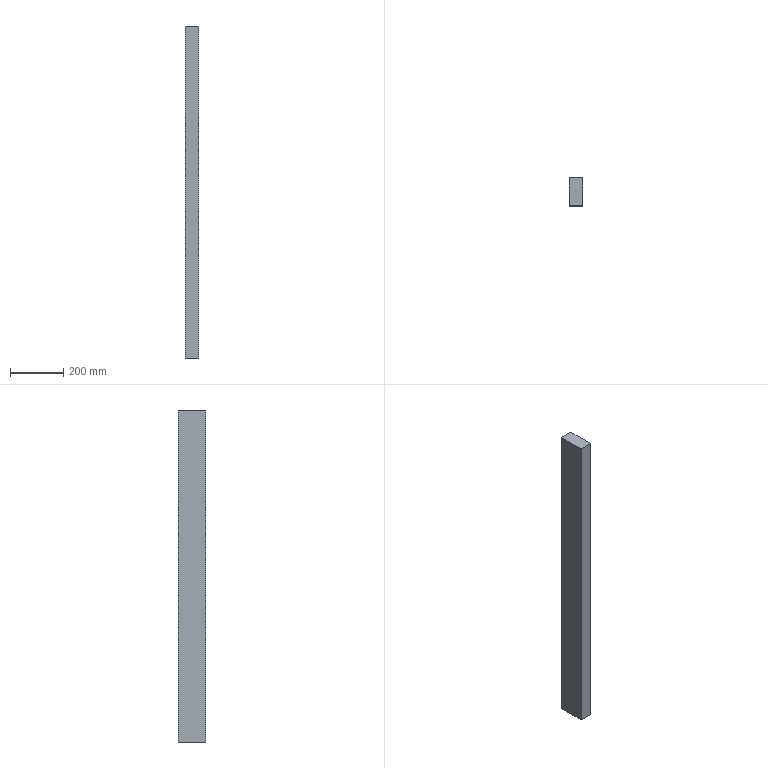Part | SolidWorks | features BaseBody 1 | 1 solid | 62 faces | box 50 x 105 x 1250 mm | volume 6548618 mm3 | cylinder 28 | cone 28 | plane 6 | commonest cylinder face diameters 5 x28
STEP:
#1=CARTESIAN_POINT('',(0.,2.5,-327.5));
#2=VERTEX_POINT('',#1);
#3=CARTESIAN_POINT('',(0.,2.5,-322.5));
#4=VERTEX_POINT('',#3);
#5=CARTESIAN_POINT('',(0.,2.5,-325.));
#6=DIRECTION('',(0.,1.,0.));
#7=DIRECTION('',(0.,0.,1.));
#8=AXIS2_PLACEMENT_3D('',#5,#6,#7);
#9=CIRCLE('',#8,2.5);
#10=EDGE_CURVE('',#2,#4,#9,.T.);
#11=ORIENTED_EDGE('',*,*,#10,.F.);
#12=CARTESIAN_POINT('',(0.,52.5,-327.5));
#13=VERTEX_POINT('',#12);
#14=CARTESIAN_POINT('',(0.,52.5,-327.5));
#15=DIRECTION('',(0.,1.,0.));
#16=VECTOR('',#15,1000.);
#17=LINE('',#14,#16);
#18=EDGE_CURVE('',#2,#13,#17,.T.);
#19=ORIENTED_EDGE('',*,*,#18,.T.);
#20=CARTESIAN_POINT('',(0.,52.5,-322.5));
#21=VERTEX_POINT('',#20);
#22=CARTESIAN_POINT('',(0.,52.5,-325.));
#23=DIRECTION('',(0.,1.,0.));
#24=DIRECTION('',(0.,0.,1.));
#25=AXIS2_PLACEMENT_3D('',#22,#23,#24);
#26=CIRCLE('',#25,2.5);
#27=EDGE_CURVE('',#13,#21,#26,.T.);
#28=ORIENTED_EDGE('',*,*,#27,.T.);
#29=CARTESIAN_POINT('',(0.,52.5,-322.5));
#30=DIRECTION('',(0.,1.,0.));
#31=VECTOR('',#30,1000.);
#32=LINE('',#29,#31);
#33=EDGE_CURVE('',#4,#21,#32,.T.);
#34=ORIENTED_EDGE('',*,*,#33,.F.);
#35=EDGE_LOOP('',(#11,#19,#28,#34));
#36=FACE_OUTER_BOUND('',#35,.T.);
#37=CARTESIAN_POINT('',(0.,52.5,-325.));
#38=DIRECTION('',(0.,1.,0.));
#39=DIRECTION('',(0.,0.,1.));
#40=AXIS2_PLACEMENT_3D('',#37,#38,#39);
#41=CYLINDRICAL_SURFACE('',#40,2.5);
#42=ADVANCED_FACE('',(#36),#41,.F.);
#43=CARTESIAN_POINT('',(0.,0.9978,-325.));
#44=VERTEX_POINT('',#43);
#45=CARTESIAN_POINT('',(0.,2.5,-322.5));
#46=DIRECTION('',(0.,0.515,0.8572));
#47=VECTOR('',#46,1000.);
#48=LINE('',#45,#47);
#49=EDGE_CURVE('',#44,#4,#48,.T.);
#50=ORIENTED_EDGE('',*,*,#49,.F.);
#51=CARTESIAN_POINT('',(0.,2.5,-327.5));
#52=DIRECTION('',(0.,0.515,-0.8572));
#53=VECTOR('',#52,1000.);
#54=LINE('',#51,#53);
#55=EDGE_CURVE('',#44,#2,#54,.T.);
#56=ORIENTED_EDGE('',*,*,#55,.T.);
#57=ORIENTED_EDGE('',*,*,#10,.T.);
#58=EDGE_LOOP('',(#50,#56,#57));
#59=FACE_OUTER_BOUND('',#58,.T.);
#60=CARTESIAN_POINT('',(0.,2.5,-325.));
#61=DIRECTION('',(0.,1.,0.));
#62=DIRECTION('',(0.,0.,1.));
#63=AXIS2_PLACEMENT_3D('',#60,#61,#62);
#64=CONICAL_SURFACE('',#63,2.5,1.03);
#65=ADVANCED_FACE('',(#59),#64,.F.);
#66=CARTESIAN_POINT('',(0.,2.5,-267.5));
#67=VERTEX_POINT('',#66);
#68=CARTESIAN_POINT('',(0.,2.5,-262.5));
#69=VERTEX_POINT('',#68);
#70=CARTESIAN_POINT('',(0.,2.5,-265.));
#71=DIRECTION('',(0.,1.,0.));
#72=DIRECTION('',(0.,0.,1.));
#73=AXIS2_PLACEMENT_3D('',#70,#71,#72);
#74=CIRCLE('',#73,2.5);
#75=EDGE_CURVE('',#67,#69,#74,.T.);
#76=ORIENTED_EDGE('',*,*,#75,.F.);
#77=CARTESIAN_POINT('',(0.,52.5,-267.5));
#78=VERTEX_POINT('',#77);
#79=CARTESIAN_POINT('',(0.,52.5,-267.5));
#80=DIRECTION('',(0.,1.,0.));
#81=VECTOR('',#80,1000.);
#82=LINE('',#79,#81);
#83=EDGE_CURVE('',#67,#78,#82,.T.);
#84=ORIENTED_EDGE('',*,*,#83,.T.);
#85=CARTESIAN_POINT('',(0.,52.5,-262.5));
#86=VERTEX_POINT('',#85);
#87=CARTESIAN_POINT('',(0.,52.5,-265.));
#88=DIRECTION('',(0.,1.,0.));
#89=DIRECTION('',(0.,0.,1.));
#90=AXIS2_PLACEMENT_3D('',#87,#88,#89);
#91=CIRCLE('',#90,2.5);
#92=EDGE_CURVE('',#78,#86,#91,.T.);
#93=ORIENTED_EDGE('',*,*,#92,.T.);
#94=CARTESIAN_POINT('',(0.,52.5,-262.5));
#95=DIRECTION('',(0.,1.,0.));
#96=VECTOR('',#95,1000.);
#97=LINE('',#94,#96);
#98=EDGE_CURVE('',#69,#86,#97,.T.);
#99=ORIENTED_EDGE('',*,*,#98,.F.);
#100=EDGE_LOOP('',(#76,#84,#93,#99));
#101=FACE_OUTER_BOUND('',#100,.T.);
#102=CARTESIAN_POINT('',(0.,52.5,-265.));
#103=DIRECTION('',(0.,1.,0.));
#104=DIRECTION('',(0.,0.,1.));
#105=AXIS2_PLACEMENT_3D('',#102,#103,#104);
#106=CYLINDRICAL_SURFACE('',#105,2.5);
#107=ADVANCED_FACE('',(#101),#106,.F.);
#108=CARTESIAN_POINT('',(0.,0.9978,-265.));
#109=VERTEX_POINT('',#108);
#110=CARTESIAN_POINT('',(0.,2.5,-262.5));
#111=DIRECTION('',(0.,0.515,0.8572));
#112=VECTOR('',#111,1000.);
#113=LINE('',#110,#112);
#114=EDGE_CURVE('',#109,#69,#113,.T.);
#115=ORIENTED_EDGE('',*,*,#114,.F.);
#116=CARTESIAN_POINT('',(0.,2.5,-267.5));
#117=DIRECTION('',(0.,0.515,-0.8572));
#118=VECTOR('',#117,1000.);
#119=LINE('',#116,#118);
#120=EDGE_CURVE('',#109,#67,#119,.T.);
#121=ORIENTED_EDGE('',*,*,#120,.T.);
#122=ORIENTED_EDGE('',*,*,#75,.T.);
#123=EDGE_LOOP('',(#115,#121,#122));
#124=FACE_OUTER_BOUND('',#123,.T.);
#125=CARTESIAN_POINT('',(0.,2.5,-265.));
#126=DIRECTION('',(0.,1.,0.));
#127=DIRECTION('',(0.,0.,1.));
#128=AXIS2_PLACEMENT_3D('',#125,#126,#127);
#129=CONICAL_SURFACE('',#128,2.5,1.03);
#130=ADVANCED_FACE('',(#124),#129,.F.);
#131=CARTESIAN_POINT('',(0.,2.5,-207.5));
#132=VERTEX_POINT('',#131);
#133=CARTESIAN_POINT('',(0.,2.5,-202.5));
#134=VERTEX_POINT('',#133);
#135=CARTESIAN_POINT('',(0.,2.5,-205.));
#136=DIRECTION('',(0.,1.,0.));
#137=DIRECTION('',(0.,0.,1.));
#138=AXIS2_PLACEMENT_3D('',#135,#136,#137);
#139=CIRCLE('',#138,2.5);
#140=EDGE_CURVE('',#132,#134,#139,.T.);
#141=ORIENTED_EDGE('',*,*,#140,.F.);
#142=CARTESIAN_POINT('',(0.,52.5,-207.5));
#143=VERTEX_POINT('',#142);
#144=CARTESIAN_POINT('',(0.,52.5,-207.5));
#145=DIRECTION('',(0.,1.,0.));
#146=VECTOR('',#145,1000.);
#147=LINE('',#144,#146);
#148=EDGE_CURVE('',#132,#143,#147,.T.);
#149=ORIENTED_EDGE('',*,*,#148,.T.);
#150=CARTESIAN_POINT('',(0.,52.5,-202.5));
#151=VERTEX_POINT('',#150);
#152=CARTESIAN_POINT('',(0.,52.5,-205.));
#153=DIRECTION('',(0.,1.,0.));
#154=DIRECTION('',(0.,0.,1.));
#155=AXIS2_PLACEMENT_3D('',#152,#153,#154);
#156=CIRCLE('',#155,2.5);
#157=EDGE_CURVE('',#143,#151,#156,.T.);
#158=ORIENTED_EDGE('',*,*,#157,.T.);
#159=CARTESIAN_POINT('',(0.,52.5,-202.5));
#160=DIRECTION('',(0.,1.,0.));
#161=VECTOR('',#160,1000.);
#162=LINE('',#159,#161);
#163=EDGE_CURVE('',#134,#151,#162,.T.);
#164=ORIENTED_EDGE('',*,*,#163,.F.);
#165=EDGE_LOOP('',(#141,#149,#158,#164));
#166=FACE_OUTER_BOUND('',#165,.T.);
#167=CARTESIAN_POINT('',(0.,52.5,-205.));
#168=DIRECTION('',(0.,1.,0.));
#169=DIRECTION('',(0.,0.,1.));
#170=AXIS2_PLACEMENT_3D('',#167,#168,#169);
#171=CYLINDRICAL_SURFACE('',#170,2.5);
#172=ADVANCED_FACE('',(#166),#171,.F.);
#173=CARTESIAN_POINT('',(0.,0.9978,-205.));
#174=VERTEX_POINT('',#173);
#175=CARTESIAN_POINT('',(0.,2.5,-202.5));
#176=DIRECTION('',(0.,0.515,0.8572));
#177=VECTOR('',#176,1000.);
#178=LINE('',#175,#177);
#179=EDGE_CURVE('',#174,#134,#178,.T.);
#180=ORIENTED_EDGE('',*,*,#179,.F.);
#181=CARTESIAN_POINT('',(0.,2.5,-207.5));
#182=DIRECTION('',(0.,0.515,-0.8572));
#183=VECTOR('',#182,1000.);
#184=LINE('',#181,#183);
#185=EDGE_CURVE('',#174,#132,#184,.T.);
#186=ORIENTED_EDGE('',*,*,#185,.T.);
#187=ORIENTED_EDGE('',*,*,#140,.T.);
#188=EDGE_LOOP('',(#180,#186,#187));
#189=FACE_OUTER_BOUND('',#188,.T.);
#190=CARTESIAN_POINT('',(0.,2.5,-205.));
#191=DIRECTION('',(0.,1.,0.));
#192=DIRECTION('',(0.,0.,1.));
#193=AXIS2_PLACEMENT_3D('',#190,#191,#192);
#194=CONICAL_SURFACE('',#193,2.5,1.03);
#195=ADVANCED_FACE('',(#189),#194,.F.);
#196=CARTESIAN_POINT('',(0.,2.5,-147.5));
#197=VERTEX_POINT('',#196);
#198=CARTESIAN_POINT('',(0.,2.5,-142.5));
#199=VERTEX_POINT('',#198);
#200=CARTESIAN_POINT('',(0.,2.5,-145.));
#201=DIRECTION('',(0.,1.,0.));
#202=DIRECTION('',(0.,0.,1.));
#203=AXIS2_PLACEMENT_3D('',#200,#201,#202);
#204=CIRCLE('',#203,2.5);
#205=EDGE_CURVE('',#197,#199,#204,.T.);
#206=ORIENTED_EDGE('',*,*,#205,.F.);
#207=CARTESIAN_POINT('',(0.,52.5,-147.5));
#208=VERTEX_POINT('',#207);
#209=CARTESIAN_POINT('',(0.,52.5,-147.5));
#210=DIRECTION('',(0.,1.,0.));
#211=VECTOR('',#210,1000.);
#212=LINE('',#209,#211);
#213=EDGE_CURVE('',#197,#208,#212,.T.);
#214=ORIENTED_EDGE('',*,*,#213,.T.);
#215=CARTESIAN_POINT('',(0.,52.5,-142.5));
#216=VERTEX_POINT('',#215);
#217=CARTESIAN_POINT('',(0.,52.5,-145.));
#218=DIRECTION('',(0.,1.,0.));
#219=DIRECTION('',(0.,0.,1.));
#220=AXIS2_PLACEMENT_3D('',#217,#218,#219);
#221=CIRCLE('',#220,2.5);
#222=EDGE_CURVE('',#208,#216,#221,.T.);
#223=ORIENTED_EDGE('',*,*,#222,.T.);
#224=CARTESIAN_POINT('',(0.,52.5,-142.5));
#225=DIRECTION('',(0.,1.,0.));
#226=VECTOR('',#225,1000.);
#227=LINE('',#224,#226);
#228=EDGE_CURVE('',#199,#216,#227,.T.);
#229=ORIENTED_EDGE('',*,*,#228,.F.);
#230=EDGE_LOOP('',(#206,#214,#223,#229));
#231=FACE_OUTER_BOUND('',#230,.T.);
#232=CARTESIAN_POINT('',(0.,52.5,-145.));
#233=DIRECTION('',(0.,1.,0.));
#234=DIRECTION('',(0.,0.,1.));
#235=AXIS2_PLACEMENT_3D('',#232,#233,#234);
#236=CYLINDRICAL_SURFACE('',#235,2.5);
#237=ADVANCED_FACE('',(#231),#236,.F.);
#238=CARTESIAN_POINT('',(0.,0.9978,-145.));
#239=VERTEX_POINT('',#238);
#240=CARTESIAN_POINT('',(0.,2.5,-142.5));
#241=DIRECTION('',(0.,0.515,0.8572));
#242=VECTOR('',#241,1000.);
#243=LINE('',#240,#242);
#244=EDGE_CURVE('',#239,#199,#243,.T.);
#245=ORIENTED_EDGE('',*,*,#244,.F.);
#246=CARTESIAN_POINT('',(0.,2.5,-147.5));
#247=DIRECTION('',(0.,0.515,-0.8572));
#248=VECTOR('',#247,1000.);
#249=LINE('',#246,#248);
#250=EDGE_CURVE('',#239,#197,#249,.T.);
#251=ORIENTED_EDGE('',*,*,#250,.T.);
#252=ORIENTED_EDGE('',*,*,#205,.T.);
#253=EDGE_LOOP('',(#245,#251,#252));
#254=FACE_OUTER_BOUND('',#253,.T.);
#255=CARTESIAN_POINT('',(0.,2.5,-145.));
#256=DIRECTION('',(0.,1.,0.));
#257=DIRECTION('',(0.,0.,1.));
#258=AXIS2_PLACEMENT_3D('',#255,#256,#257);
#259=CONICAL_SURFACE('',#258,2.5,1.03);
#260=ADVANCED_FACE('',(#254),#259,.F.);
#261=CARTESIAN_POINT('',(0.,2.5,-87.5));
#262=VERTEX_POINT('',#261);
#263=CARTESIAN_POINT('',(0.,2.5,-82.5));
#264=VERTEX_POINT('',#263);
#265=CARTESIAN_POINT('',(0.,2.5,-85.));
#266=DIRECTION('',(0.,1.,0.));
#267=DIRECTION('',(0.,0.,1.));
#268=AXIS2_PLACEMENT_3D('',#265,#266,#267);
#269=CIRCLE('',#268,2.5);
#270=EDGE_CURVE('',#262,#264,#269,.T.);
#271=ORIENTED_EDGE('',*,*,#270,.F.);
#272=CARTESIAN_POINT('',(0.,52.5,-87.5));
#273=VERTEX_POINT('',#272);
#274=CARTESIAN_POINT('',(0.,52.5,-87.5));
#275=DIRECTION('',(0.,1.,0.));
#276=VECTOR('',#275,1000.);
#277=LINE('',#274,#276);
#278=EDGE_CURVE('',#262,#273,#277,.T.);
#279=ORIENTED_EDGE('',*,*,#278,.T.);
#280=CARTESIAN_POINT('',(0.,52.5,-82.5));
#281=VERTEX_POINT('',#280);
#282=CARTESIAN_POINT('',(0.,52.5,-85.));
#283=DIRECTION('',(0.,1.,0.));
#284=DIRECTION('',(0.,0.,1.));
#285=AXIS2_PLACEMENT_3D('',#282,#283,#284);
#286=CIRCLE('',#285,2.5);
#287=EDGE_CURVE('',#273,#281,#286,.T.);
#288=ORIENTED_EDGE('',*,*,#287,.T.);
#289=CARTESIAN_POINT('',(0.,52.5,-82.5));
#290=DIRECTION('',(0.,1.,0.));
#291=VECTOR('',#290,1000.);
#292=LINE('',#289,#291);
#293=EDGE_CURVE('',#264,#281,#292,.T.);
#294=ORIENTED_EDGE('',*,*,#293,.F.);
#295=EDGE_LOOP('',(#271,#279,#288,#294));
#296=FACE_OUTER_BOUND('',#295,.T.);
#297=CARTESIAN_POINT('',(0.,52.5,-85.));
#298=DIRECTION('',(0.,1.,0.));
#299=DIRECTION('',(0.,0.,1.));
#300=AXIS2_PLACEMENT_3D('',#297,#298,#299);
#301=CYLINDRICAL_SURFACE('',#300,2.5);
#302=ADVANCED_FACE('',(#296),#301,.F.);
#303=CARTESIAN_POINT('',(0.,0.9978,-85.));
#304=VERTEX_POINT('',#303);
#305=CARTESIAN_POINT('',(0.,2.5,-82.5));
#306=DIRECTION('',(0.,0.515,0.8572));
#307=VECTOR('',#306,1000.);
#308=LINE('',#305,#307);
#309=EDGE_CURVE('',#304,#264,#308,.T.);
#310=ORIENTED_EDGE('',*,*,#309,.F.);
#311=CARTESIAN_POINT('',(0.,2.5,-87.5));
#312=DIRECTION('',(0.,0.515,-0.8572));
#313=VECTOR('',#312,1000.);
#314=LINE('',#311,#313);
#315=EDGE_CURVE('',#304,#262,#314,.T.);
#316=ORIENTED_EDGE('',*,*,#315,.T.);
#317=ORIENTED_EDGE('',*,*,#270,.T.);
#318=EDGE_LOOP('',(#310,#316,#317));
#319=FACE_OUTER_BOUND('',#318,.T.);
#320=CARTESIAN_POINT('',(0.,2.5,-85.));
#321=DIRECTION('',(0.,1.,0.));
#322=DIRECTION('',(0.,0.,1.));
#323=AXIS2_PLACEMENT_3D('',#320,#321,#322);
#324=CONICAL_SURFACE('',#323,2.5,1.03);
#325=ADVANCED_FACE('',(#319),#324,.F.);
#326=CARTESIAN_POINT('',(0.,2.5,-27.5));
#327=VERTEX_POINT('',#326);
#328=CARTESIAN_POINT('',(0.,2.5,-22.5));
#329=VERTEX_POINT('',#328);
#330=CARTESIAN_POINT('',(0.,2.5,-25.));
#331=DIRECTION('',(0.,1.,0.));
#332=DIRECTION('',(0.,0.,1.));
#333=AXIS2_PLACEMENT_3D('',#330,#331,#332);
#334=CIRCLE('',#333,2.5);
#335=EDGE_CURVE('',#327,#329,#334,.T.);
#336=ORIENTED_EDGE('',*,*,#335,.F.);
#337=CARTESIAN_POINT('',(0.,52.5,-27.5));
#338=VERTEX_POINT('',#337);
#339=CARTESIAN_POINT('',(0.,52.5,-27.5));
#340=DIRECTION('',(0.,1.,0.));
#341=VECTOR('',#340,1000.);
#342=LINE('',#339,#341);
#343=EDGE_CURVE('',#327,#338,#342,.T.);
#344=ORIENTED_EDGE('',*,*,#343,.T.);
#345=CARTESIAN_POINT('',(0.,52.5,-22.5));
#346=VERTEX_POINT('',#345);
#347=CARTESIAN_POINT('',(0.,52.5,-25.));
#348=DIRECTION('',(0.,1.,0.));
#349=DIRECTION('',(0.,0.,1.));
#350=AXIS2_PLACEMENT_3D('',#347,#348,#349);
#351=CIRCLE('',#350,2.5);
#352=EDGE_CURVE('',#338,#346,#351,.T.);
#353=ORIENTED_EDGE('',*,*,#352,.T.);
#354=CARTESIAN_POINT('',(0.,52.5,-22.5));
#355=DIRECTION('',(0.,1.,0.));
#356=VECTOR('',#355,1000.);
#357=LINE('',#354,#356);
#358=EDGE_CURVE('',#329,#346,#357,.T.);
#359=ORIENTED_EDGE('',*,*,#358,.F.);
#360=EDGE_LOOP('',(#336,#344,#353,#359));
#361=FACE_OUTER_BOUND('',#360,.T.);
#362=CARTESIAN_POINT('',(0.,52.5,-25.));
#363=DIRECTION('',(0.,1.,0.));
#364=DIRECTION('',(0.,0.,1.));
#365=AXIS2_PLACEMENT_3D('',#362,#363,#364);
#366=CYLINDRICAL_SURFACE('',#365,2.5);
#367=ADVANCED_FACE('',(#361),#366,.F.);
#368=CARTESIAN_POINT('',(0.,0.9978,-25.));
#369=VERTEX_POINT('',#368);
#370=CARTESIAN_POINT('',(0.,2.5,-22.5));
#371=DIRECTION('',(0.,0.515,0.8572));
#372=VECTOR('',#371,1000.);
#373=LINE('',#370,#372);
#374=EDGE_CURVE('',#369,#329,#373,.T.);
#375=ORIENTED_EDGE('',*,*,#374,.F.);
#376=CARTESIAN_POINT('',(0.,2.5,-27.5));
#377=DIRECTION('',(0.,0.515,-0.8572));
#378=VECTOR('',#377,1000.);
#379=LINE('',#376,#378);
#380=EDGE_CURVE('',#369,#327,#379,.T.);
#381=ORIENTED_EDGE('',*,*,#380,.T.);
#382=ORIENTED_EDGE('',*,*,#335,.T.);
#383=EDGE_LOOP('',(#375,#381,#382));
#384=FACE_OUTER_BOUND('',#383,.T.);
#385=CARTESIAN_POINT('',(0.,2.5,-25.));
#386=DIRECTION('',(0.,1.,0.));
#387=DIRECTION('',(0.,0.,1.));
#388=AXIS2_PLACEMENT_3D('',#385,#386,#387);
#389=CONICAL_SURFACE('',#388,2.5,1.03);
#390=ADVANCED_FACE('',(#384),#389,.F.);
#391=CARTESIAN_POINT('',(0.,2.5,32.5));
#392=VERTEX_POINT('',#391);
#393=CARTESIAN_POINT('',(0.,2.5,37.5));
#394=VERTEX_POINT('',#393);
#395=CARTESIAN_POINT('',(0.,2.5,35.));
#396=DIRECTION('',(0.,1.,0.));
#397=DIRECTION('',(0.,0.,1.));
#398=AXIS2_PLACEMENT_3D('',#395,#396,#397);
#399=CIRCLE('',#398,2.5);
#400=EDGE_CURVE('',#392,#394,#399,.T.);
#401=ORIENTED_EDGE('',*,*,#400,.F.);
#402=CARTESIAN_POINT('',(0.,52.5,32.5));
#403=VERTEX_POINT('',#402);
#404=CARTESIAN_POINT('',(0.,52.5,32.5));
#405=DIRECTION('',(0.,1.,0.));
#406=VECTOR('',#405,1000.);
#407=LINE('',#404,#406);
#408=EDGE_CURVE('',#392,#403,#407,.T.);
#409=ORIENTED_EDGE('',*,*,#408,.T.);
#410=CARTESIAN_POINT('',(0.,52.5,37.5));
#411=VERTEX_POINT('',#410);
#412=CARTESIAN_POINT('',(0.,52.5,35.));
#413=DIRECTION('',(0.,1.,0.));
#414=DIRECTION('',(0.,0.,1.));
#415=AXIS2_PLACEMENT_3D('',#412,#413,#414);
#416=CIRCLE('',#415,2.5);
#417=EDGE_CURVE('',#403,#411,#416,.T.);
#418=ORIENTED_EDGE('',*,*,#417,.T.);
#419=CARTESIAN_POINT('',(0.,52.5,37.5));
#420=DIRECTION('',(0.,1.,0.));
#421=VECTOR('',#420,1000.);
#422=LINE('',#419,#421);
#423=EDGE_CURVE('',#394,#411,#422,.T.);
#424=ORIENTED_EDGE('',*,*,#423,.F.);
#425=EDGE_LOOP('',(#401,#409,#418,#424));
#426=FACE_OUTER_BOUND('',#425,.T.);
#427=CARTESIAN_POINT('',(0.,52.5,35.));
#428=DIRECTION('',(0.,1.,0.));
#429=DIRECTION('',(0.,0.,1.));
#430=AXIS2_PLACEMENT_3D('',#427,#428,#429);
#431=CYLINDRICAL_SURFACE('',#430,2.5);
#432=ADVANCED_FACE('',(#426),#431,.F.);
#433=CARTESIAN_POINT('',(0.,0.9978,35.));
#434=VERTEX_POINT('',#433);
#435=CARTESIAN_POINT('',(0.,2.5,37.5));
#436=DIRECTION('',(0.,0.515,0.8572));
#437=VECTOR('',#436,1000.);
#438=LINE('',#435,#437);
#439=EDGE_CURVE('',#434,#394,#438,.T.);
#440=ORIENTED_EDGE('',*,*,#439,.F.);
#441=CARTESIAN_POINT('',(0.,2.5,32.5));
#442=DIRECTION('',(0.,0.515,-0.8572));
#443=VECTOR('',#442,1000.);
#444=LINE('',#441,#443);
#445=EDGE_CURVE('',#434,#392,#444,.T.);
#446=ORIENTED_EDGE('',*,*,#445,.T.);
#447=ORIENTED_EDGE('',*,*,#400,.T.);
#448=EDGE_LOOP('',(#440,#446,#447));
#449=FACE_OUTER_BOUND('',#448,.T.);
#450=CARTESIAN_POINT('',(0.,2.5,35.));
#451=DIRECTION('',(0.,1.,0.));
#452=DIRECTION('',(0.,0.,1.));
#453=AXIS2_PLACEMENT_3D('',#450,#451,#452);
#454=CONICAL_SURFACE('',#453,2.5,1.03);
#455=ADVANCED_FACE('',(#449),#454,.F.);
#456=CARTESIAN_POINT('',(0.,2.5,92.5));
#457=VERTEX_POINT('',#456);
#458=CARTESIAN_POINT('',(0.,2.5,97.5));
#459=VERTEX_POINT('',#458);
#460=CARTESIAN_POINT('',(0.,2.5,95.));
#461=DIRECTION('',(0.,1.,0.));
#462=DIRECTION('',(0.,0.,1.));
#463=AXIS2_PLACEMENT_3D('',#460,#461,#462);
#464=CIRCLE('',#463,2.5);
#465=EDGE_CURVE('',#457,#459,#464,.T.);
#466=ORIENTED_EDGE('',*,*,#465,.F.);
#467=CARTESIAN_POINT('',(0.,52.5,92.5));
#468=VERTEX_POINT('',#467);
#469=CARTESIAN_POINT('',(0.,52.5,92.5));
#470=DIRECTION('',(0.,1.,0.));
#471=VECTOR('',#470,1000.);
#472=LINE('',#469,#471);
#473=EDGE_CURVE('',#457,#468,#472,.T.);
#474=ORIENTED_EDGE('',*,*,#473,.T.);
#475=CARTESIAN_POINT('',(0.,52.5,97.5));
#476=VERTEX_POINT('',#475);
#477=CARTESIAN_POINT('',(0.,52.5,95.));
#478=DIRECTION('',(0.,1.,0.));
#479=DIRECTION('',(0.,0.,1.));
#480=AXIS2_PLACEMENT_3D('',#477,#478,#479);
#481=CIRCLE('',#480,2.5);
#482=EDGE_CURVE('',#468,#476,#481,.T.);
#483=ORIENTED_EDGE('',*,*,#482,.T.);
#484=CARTESIAN_POINT('',(0.,52.5,97.5));
#485=DIRECTION('',(0.,1.,0.));
#486=VECTOR('',#485,1000.);
#487=LINE('',#484,#486);
#488=EDGE_CURVE('',#459,#476,#487,.T.);
#489=ORIENTED_EDGE('',*,*,#488,.F.);
#490=EDGE_LOOP('',(#466,#474,#483,#489));
#491=FACE_OUTER_BOUND('',#490,.T.);
#492=CARTESIAN_POINT('',(0.,52.5,95.));
#493=DIRECTION('',(0.,1.,0.));
#494=DIRECTION('',(0.,0.,1.));
#495=AXIS2_PLACEMENT_3D('',#492,#493,#494);
#496=CYLINDRICAL_SURFACE('',#495,2.5);
#497=ADVANCED_FACE('',(#491),#496,.F.);
#498=CARTESIAN_POINT('',(0.,0.9978,95.));
#499=VERTEX_POINT('',#498);
#500=CARTESIAN_POINT('',(0.,2.5,97.5));
#501=DIRECTION('',(0.,0.515,0.8572));
#502=VECTOR('',#501,1000.);
#503=LINE('',#500,#502);
#504=EDGE_CURVE('',#499,#459,#503,.T.);
#505=ORIENTED_EDGE('',*,*,#504,.F.);
#506=CARTESIAN_POINT('',(0.,2.5,92.5));
#507=DIRECTION('',(0.,0.515,-0.8572));
#508=VECTOR('',#507,1000.);
#509=LINE('',#506,#508);
#510=EDGE_CURVE('',#499,#457,#509,.T.);
#511=ORIENTED_EDGE('',*,*,#510,.T.);
#512=ORIENTED_EDGE('',*,*,#465,.T.);
#513=EDGE_LOOP('',(#505,#511,#512));
#514=FACE_OUTER_BOUND('',#513,.T.);
#515=CARTESIAN_POINT('',(0.,2.5,95.));
#516=DIRECTION('',(0.,1.,0.));
#517=DIRECTION('',(0.,0.,1.));
#518=AXIS2_PLACEMENT_3D('',#515,#516,#517);
#519=CONICAL_SURFACE('',#518,2.5,1.03);
#520=ADVANCED_FACE('',(#514),#519,.F.);
#521=CARTESIAN_POINT('',(0.,2.5,152.5));
#522=VERTEX_POINT('',#521);
#523=CARTESIAN_POINT('',(0.,2.5,157.5));
#524=VERTEX_POINT('',#523);
#525=CARTESIAN_POINT('',(0.,2.5,155.));
#526=DIRECTION('',(0.,1.,0.));
#527=DIRECTION('',(0.,0.,1.));
#528=AXIS2_PLACEMENT_3D('',#525,#526,#527);
#529=CIRCLE('',#528,2.5);
#530=EDGE_CURVE('',#522,#524,#529,.T.);
#531=ORIENTED_EDGE('',*,*,#530,.F.);
#532=CARTESIAN_POINT('',(0.,52.5,152.5));
#533=VERTEX_POINT('',#532);
#534=CARTESIAN_POINT('',(0.,52.5,152.5));
#535=DIRECTION('',(0.,1.,0.));
#536=VECTOR('',#535,1000.);
#537=LINE('',#534,#536);
#538=EDGE_CURVE('',#522,#533,#537,.T.);
#539=ORIENTED_EDGE('',*,*,#538,.T.);
#540=CARTESIAN_POINT('',(0.,52.5,157.5));
#541=VERTEX_POINT('',#540);
#542=CARTESIAN_POINT('',(0.,52.5,155.));
#543=DIRECTION('',(0.,1.,0.));
#544=DIRECTION('',(0.,0.,1.));
#545=AXIS2_PLACEMENT_3D('',#542,#543,#544);
#546=CIRCLE('',#545,2.5);
#547=EDGE_CURVE('',#533,#541,#546,.T.);
#548=ORIENTED_EDGE('',*,*,#547,.T.);
#549=CARTESIAN_POINT('',(0.,52.5,157.5));
#550=DIRECTION('',(0.,1.,0.));
#551=VECTOR('',#550,1000.);
#552=LINE('',#549,#551);
#553=EDGE_CURVE('',#524,#541,#552,.T.);
#554=ORIENTED_EDGE('',*,*,#553,.F.);
#555=EDGE_LOOP('',(#531,#539,#548,#554));
#556=FACE_OUTER_BOUND('',#555,.T.);
#557=CARTESIAN_POINT('',(0.,52.5,155.));
#558=DIRECTION('',(0.,1.,0.));
#559=DIRECTION('',(0.,0.,1.));
#560=AXIS2_PLACEMENT_3D('',#557,#558,#559);
#561=CYLINDRICAL_SURFACE('',#560,2.5);
#562=ADVANCED_FACE('',(#556),#561,.F.);
#563=CARTESIAN_POINT('',(0.,0.9978,155.));
#564=VERTEX_POINT('',#563);
#565=CARTESIAN_POINT('',(0.,2.5,157.5));
#566=DIRECTION('',(0.,0.515,0.8572));
#567=VECTOR('',#566,1000.);
#568=LINE('',#565,#567);
#569=EDGE_CURVE('',#564,#524,#568,.T.);
#570=ORIENTED_EDGE('',*,*,#569,.F.);
#571=CARTESIAN_POINT('',(0.,2.5,152.5));
#572=DIRECTION('',(0.,0.515,-0.8572));
#573=VECTOR('',#572,1000.);
#574=LINE('',#571,#573);
#575=EDGE_CURVE('',#564,#522,#574,.T.);
#576=ORIENTED_EDGE('',*,*,#575,.T.);
#577=ORIENTED_EDGE('',*,*,#530,.T.);
#578=EDGE_LOOP('',(#570,#576,#577));
#579=FACE_OUTER_BOUND('',#578,.T.);
#580=CARTESIAN_POINT('',(0.,2.5,155.));
#581=DIRECTION('',(0.,1.,0.));
#582=DIRECTION('',(0.,0.,1.));
#583=AXIS2_PLACEMENT_3D('',#580,#581,#582);
#584=CONICAL_SURFACE('',#583,2.5,1.03);
#585=ADVANCED_FACE('',(#579),#584,.F.);
#586=CARTESIAN_POINT('',(0.,2.5,212.5));
#587=VERTEX_POINT('',#586);
#588=CARTESIAN_POINT('',(0.,2.5,217.5));
#589=VERTEX_POINT('',#588);
#590=CARTESIAN_POINT('',(0.,2.5,215.));
#591=DIRECTION('',(0.,1.,0.));
#592=DIRECTION('',(0.,0.,1.));
#593=AXIS2_PLACEMENT_3D('',#590,#591,#592);
#594=CIRCLE('',#593,2.5);
#595=EDGE_CURVE('',#587,#589,#594,.T.);
#596=ORIENTED_EDGE('',*,*,#595,.F.);
#597=CARTESIAN_POINT('',(0.,52.5,212.5));
#598=VERTEX_POINT('',#597);
#599=CARTESIAN_POINT('',(0.,52.5,212.5));
#600=DIRECTION('',(0.,1.,0.));
#601=VECTOR('',#600,1000.);
#602=LINE('',#599,#601);
#603=EDGE_CURVE('',#587,#598,#602,.T.);
#604=ORIENTED_EDGE('',*,*,#603,.T.);
#605=CARTESIAN_POINT('',(0.,52.5,217.5));
#606=VERTEX_POINT('',#605);
#607=CARTESIAN_POINT('',(0.,52.5,215.));
#608=DIRECTION('',(0.,1.,0.));
#609=DIRECTION('',(0.,0.,1.));
#610=AXIS2_PLACEMENT_3D('',#607,#608,#609);
#611=CIRCLE('',#610,2.5);
#612=EDGE_CURVE('',#598,#606,#611,.T.);
#613=ORIENTED_EDGE('',*,*,#612,.T.);
#614=CARTESIAN_POINT('',(0.,52.5,217.5));
#615=DIRECTION('',(0.,1.,0.));
#616=VECTOR('',#615,1000.);
#617=LINE('',#614,#616);
#618=EDGE_CURVE('',#589,#606,#617,.T.);
#619=ORIENTED_EDGE('',*,*,#618,.F.);
#620=EDGE_LOOP('',(#596,#604,#613,#619));
#621=FACE_OUTER_BOUND('',#620,.T.);
#622=CARTESIAN_POINT('',(0.,52.5,215.));
#623=DIRECTION('',(0.,1.,0.));
#624=DIRECTION('',(0.,0.,1.));
#625=AXIS2_PLACEMENT_3D('',#622,#623,#624);
#626=CYLINDRICAL_SURFACE('',#625,2.5);
#627=ADVANCED_FACE('',(#621),#626,.F.);
#628=CARTESIAN_POINT('',(0.,0.9978,215.));
#629=VERTEX_POINT('',#628);
#630=CARTESIAN_POINT('',(0.,2.5,217.5));
#631=DIRECTION('',(0.,0.515,0.8572));
#632=VECTOR('',#631,1000.);
#633=LINE('',#630,#632);
#634=EDGE_CURVE('',#629,#589,#633,.T.);
#635=ORIENTED_EDGE('',*,*,#634,.F.);
#636=CARTESIAN_POINT('',(0.,2.5,212.5));
#637=DIRECTION('',(0.,0.515,-0.8572));
#638=VECTOR('',#637,1000.);
#639=LINE('',#636,#638);
#640=EDGE_CURVE('',#629,#587,#639,.T.);
#641=ORIENTED_EDGE('',*,*,#640,.T.);
#642=ORIENTED_EDGE('',*,*,#595,.T.);
#643=EDGE_LOOP('',(#635,#641,#642));
#644=FACE_OUTER_BOUND('',#643,.T.);
#645=CARTESIAN_POINT('',(0.,2.5,215.));
#646=DIRECTION('',(0.,1.,0.));
#647=DIRECTION('',(0.,0.,1.));
#648=AXIS2_PLACEMENT_3D('',#645,#646,#647);
#649=CONICAL_SURFACE('',#648,2.5,1.03);
#650=ADVANCED_FACE('',(#644),#649,.F.);
#651=CARTESIAN_POINT('',(0.,2.5,272.5));
#652=VERTEX_POINT('',#651);
#653=CARTESIAN_POINT('',(0.,2.5,277.5));
#654=VERTEX_POINT('',#653);
#655=CARTESIAN_POINT('',(0.,2.5,275.));
#656=DIRECTION('',(0.,1.,0.));
#657=DIRECTION('',(0.,0.,1.));
#658=AXIS2_PLACEMENT_3D('',#655,#656,#657);
#659=CIRCLE('',#658,2.5);
#660=EDGE_CURVE('',#652,#654,#659,.T.);
#661=ORIENTED_EDGE('',*,*,#660,.F.);
#662=CARTESIAN_POINT('',(0.,52.5,272.5));
#663=VERTEX_POINT('',#662);
#664=CARTESIAN_POINT('',(0.,52.5,272.5));
#665=DIRECTION('',(0.,1.,0.));
#666=VECTOR('',#665,1000.);
#667=LINE('',#664,#666);
#668=EDGE_CURVE('',#652,#663,#667,.T.);
#669=ORIENTED_EDGE('',*,*,#668,.T.);
#670=CARTESIAN_POINT('',(0.,52.5,277.5));
#671=VERTEX_POINT('',#670);
#672=CARTESIAN_POINT('',(0.,52.5,275.));
#673=DIRECTION('',(0.,1.,0.));
#674=DIRECTION('',(0.,0.,1.));
#675=AXIS2_PLACEMENT_3D('',#672,#673,#674);
#676=CIRCLE('',#675,2.5);
#677=EDGE_CURVE('',#663,#671,#676,.T.);
#678=ORIENTED_EDGE('',*,*,#677,.T.);
#679=CARTESIAN_POINT('',(0.,52.5,277.5));
#680=DIRECTION('',(0.,1.,0.));
#681=VECTOR('',#680,1000.);
#682=LINE('',#679,#681);
#683=EDGE_CURVE('',#654,#671,#682,.T.);
#684=ORIENTED_EDGE('',*,*,#683,.F.);
#685=EDGE_LOOP('',(#661,#669,#678,#684));
#686=FACE_OUTER_BOUND('',#685,.T.);
#687=CARTESIAN_POINT('',(0.,52.5,275.));
#688=DIRECTION('',(0.,1.,0.));
#689=DIRECTION('',(0.,0.,1.));
#690=AXIS2_PLACEMENT_3D('',#687,#688,#689);
#691=CYLINDRICAL_SURFACE('',#690,2.5);
#692=ADVANCED_FACE('',(#686),#691,.F.);
#693=CARTESIAN_POINT('',(0.,0.9978,275.));
#694=VERTEX_POINT('',#693);
#695=CARTESIAN_POINT('',(0.,2.5,277.5));
#696=DIRECTION('',(0.,0.515,0.8572));
#697=VECTOR('',#696,1000.);
#698=LINE('',#695,#697);
#699=EDGE_CURVE('',#694,#654,#698,.T.);
#700=ORIENTED_EDGE('',*,*,#699,.F.);
#701=CARTESIAN_POINT('',(0.,2.5,272.5));
#702=DIRECTION('',(0.,0.515,-0.8572));
#703=VECTOR('',#702,1000.);
#704=LINE('',#701,#703);
#705=EDGE_CURVE('',#694,#652,#704,.T.);
#706=ORIENTED_EDGE('',*,*,#705,.T.);
#707=ORIENTED_EDGE('',*,*,#660,.T.);
#708=EDGE_LOOP('',(#700,#706,#707));
#709=FACE_OUTER_BOUND('',#708,.T.);
#710=CARTESIAN_POINT('',(0.,2.5,275.));
#711=DIRECTION('',(0.,1.,0.));
#712=DIRECTION('',(0.,0.,1.));
#713=AXIS2_PLACEMENT_3D('',#710,#711,#712);
#714=CONICAL_SURFACE('',#713,2.5,1.03);
#715=ADVANCED_FACE('',(#709),#714,.F.);
#716=CARTESIAN_POINT('',(0.,2.5,332.5));
#717=VERTEX_POINT('',#716);
#718=CARTESIAN_POINT('',(0.,2.5,337.5));
#719=VERTEX_POINT('',#718);
#720=CARTESIAN_POINT('',(0.,2.5,335.));
#721=DIRECTION('',(0.,1.,0.));
#722=DIRECTION('',(0.,0.,1.));
#723=AXIS2_PLACEMENT_3D('',#720,#721,#722);
#724=CIRCLE('',#723,2.5);
#725=EDGE_CURVE('',#717,#719,#724,.T.);
#726=ORIENTED_EDGE('',*,*,#725,.F.);
#727=CARTESIAN_POINT('',(0.,52.5,332.5));
#728=VERTEX_POINT('',#727);
#729=CARTESIAN_POINT('',(0.,52.5,332.5));
#730=DIRECTION('',(0.,1.,0.));
#731=VECTOR('',#730,1000.);
#732=LINE('',#729,#731);
#733=EDGE_CURVE('',#717,#728,#732,.T.);
#734=ORIENTED_EDGE('',*,*,#733,.T.);
#735=CARTESIAN_POINT('',(0.,52.5,337.5));
#736=VERTEX_POINT('',#735);
#737=CARTESIAN_POINT('',(0.,52.5,335.));
#738=DIRECTION('',(0.,1.,0.));
#739=DIRECTION('',(0.,0.,1.));
#740=AXIS2_PLACEMENT_3D('',#737,#738,#739);
#741=CIRCLE('',#740,2.5);
#742=EDGE_CURVE('',#728,#736,#741,.T.);
#743=ORIENTED_EDGE('',*,*,#742,.T.);
#744=CARTESIAN_POINT('',(0.,52.5,337.5));
#745=DIRECTION('',(0.,1.,0.));
#746=VECTOR('',#745,1000.);
#747=LINE('',#744,#746);
#748=EDGE_CURVE('',#719,#736,#747,.T.);
#749=ORIENTED_EDGE('',*,*,#748,.F.);
#750=EDGE_LOOP('',(#726,#734,#743,#749));
#751=FACE_OUTER_BOUND('',#750,.T.);
#752=CARTESIAN_POINT('',(0.,52.5,335.));
#753=DIRECTION('',(0.,1.,0.));
#754=DIRECTION('',(0.,0.,1.));
#755=AXIS2_PLACEMENT_3D('',#752,#753,#754);
#756=CYLINDRICAL_SURFACE('',#755,2.5);
#757=ADVANCED_FACE('',(#751),#756,.F.);
#758=CARTESIAN_POINT('',(0.,0.9978,335.));
#759=VERTEX_POINT('',#758);
#760=CARTESIAN_POINT('',(0.,2.5,337.5));
#761=DIRECTION('',(0.,0.515,0.8572));
#762=VECTOR('',#761,1000.);
#763=LINE('',#760,#762);
#764=EDGE_CURVE('',#759,#719,#763,.T.);
#765=ORIENTED_EDGE('',*,*,#764,.F.);
#766=CARTESIAN_POINT('',(0.,2.5,332.5));
#767=DIRECTION('',(0.,0.515,-0.8572));
#768=VECTOR('',#767,1000.);
#769=LINE('',#766,#768);
#770=EDGE_CURVE('',#759,#717,#769,.T.);
#771=ORIENTED_EDGE('',*,*,#770,.T.);
#772=ORIENTED_EDGE('',*,*,#725,.T.);
#773=EDGE_LOOP('',(#765,#771,#772));
#774=FACE_OUTER_BOUND('',#773,.T.);
#775=CARTESIAN_POINT('',(0.,2.5,335.));
#776=DIRECTION('',(0.,1.,0.));
#777=DIRECTION('',(0.,0.,1.));
#778=AXIS2_PLACEMENT_3D('',#775,#776,#777);
#779=CONICAL_SURFACE('',#778,2.5,1.03);
#780=ADVANCED_FACE('',(#774),#779,.F.);
#781=CARTESIAN_POINT('',(0.,2.5,452.5));
#782=VERTEX_POINT('',#781);
#783=CARTESIAN_POINT('',(0.,2.5,457.5));
#784=VERTEX_POINT('',#783);
#785=CARTESIAN_POINT('',(0.,2.5,455.));
#786=DIRECTION('',(0.,1.,0.));
#787=DIRECTION('',(0.,0.,1.));
#788=AXIS2_PLACEMENT_3D('',#785,#786,#787);
#789=CIRCLE('',#788,2.5);
#790=EDGE_CURVE('',#782,#784,#789,.T.);
#791=ORIENTED_EDGE('',*,*,#790,.F.);
#792=CARTESIAN_POINT('',(0.,52.5,452.5));
#793=VERTEX_POINT('',#792);
#794=CARTESIAN_POINT('',(0.,52.5,452.5));
#795=DIRECTION('',(0.,1.,0.));
#796=VECTOR('',#795,1000.);
#797=LINE('',#794,#796);
#798=EDGE_CURVE('',#782,#793,#797,.T.);
#799=ORIENTED_EDGE('',*,*,#798,.T.);
#800=CARTESIAN_POINT('',(0.,52.5,457.5));
#801=VERTEX_POINT('',#800);
#802=CARTESIAN_POINT('',(0.,52.5,455.));
#803=DIRECTION('',(0.,1.,0.));
#804=DIRECTION('',(0.,0.,1.));
#805=AXIS2_PLACEMENT_3D('',#802,#803,#804);
#806=CIRCLE('',#805,2.5);
#807=EDGE_CURVE('',#793,#801,#806,.T.);
#808=ORIENTED_EDGE('',*,*,#807,.T.);
#809=CARTESIAN_POINT('',(0.,52.5,457.5));
#810=DIRECTION('',(0.,1.,0.));
#811=VECTOR('',#810,1000.);
#812=LINE('',#809,#811);
#813=EDGE_CURVE('',#784,#801,#812,.T.);
#814=ORIENTED_EDGE('',*,*,#813,.F.);
#815=EDGE_LOOP('',(#791,#799,#808,#814));
#816=FACE_OUTER_BOUND('',#815,.T.);
#817=CARTESIAN_POINT('',(0.,52.5,455.));
#818=DIRECTION('',(0.,1.,0.));
#819=DIRECTION('',(0.,0.,1.));
#820=AXIS2_PLACEMENT_3D('',#817,#818,#819);
#821=CYLINDRICAL_SURFACE('',#820,2.5);
#822=ADVANCED_FACE('',(#816),#821,.F.);
#823=CARTESIAN_POINT('',(0.,0.9978,455.));
#824=VERTEX_POINT('',#823);
#825=CARTESIAN_POINT('',(0.,2.5,457.5));
#826=DIRECTION('',(0.,0.515,0.8572));
#827=VECTOR('',#826,1000.);
#828=LINE('',#825,#827);
#829=EDGE_CURVE('',#824,#784,#828,.T.);
#830=ORIENTED_EDGE('',*,*,#829,.F.);
#831=CARTESIAN_POINT('',(0.,2.5,452.5));
#832=DIRECTION('',(0.,0.515,-0.8572));
#833=VECTOR('',#832,1000.);
#834=LINE('',#831,#833);
#835=EDGE_CURVE('',#824,#782,#834,.T.);
#836=ORIENTED_EDGE('',*,*,#835,.T.);
#837=ORIENTED_EDGE('',*,*,#790,.T.);
#838=EDGE_LOOP('',(#830,#836,#837));
#839=FACE_OUTER_BOUND('',#838,.T.);
#840=CARTESIAN_POINT('',(0.,2.5,455.));
#841=DIRECTION('',(0.,1.,0.));
#842=DIRECTION('',(0.,0.,1.));
#843=AXIS2_PLACEMENT_3D('',#840,#841,#842);
#844=CONICAL_SURFACE('',#843,2.5,1.03);
#845=ADVANCED_FACE('',(#839),#844,.F.);
#846=CARTESIAN_POINT('',(0.,2.5,392.5));
#847=VERTEX_POINT('',#846);
#848=CARTESIAN_POINT('',(0.,2.5,397.5));
#849=VERTEX_POINT('',#848);
#850=CARTESIAN_POINT('',(0.,2.5,395.));
#851=DIRECTION('',(0.,1.,0.));
#852=DIRECTION('',(0.,0.,1.));
#853=AXIS2_PLACEMENT_3D('',#850,#851,#852);
#854=CIRCLE('',#853,2.5);
#855=EDGE_CURVE('',#847,#849,#854,.T.);
#856=ORIENTED_EDGE('',*,*,#855,.F.);
#857=CARTESIAN_POINT('',(0.,52.5,392.5));
#858=VERTEX_POINT('',#857);
#859=CARTESIAN_POINT('',(0.,52.5,392.5));
#860=DIRECTION('',(0.,1.,0.));
#861=VECTOR('',#860,1000.);
#862=LINE('',#859,#861);
#863=EDGE_CURVE('',#847,#858,#862,.T.);
#864=ORIENTED_EDGE('',*,*,#863,.T.);
#865=CARTESIAN_POINT('',(0.,52.5,397.5));
#866=VERTEX_POINT('',#865);
#867=CARTESIAN_POINT('',(0.,52.5,395.));
#868=DIRECTION('',(0.,1.,0.));
#869=DIRECTION('',(0.,0.,1.));
#870=AXIS2_PLACEMENT_3D('',#867,#868,#869);
#871=CIRCLE('',#870,2.5);
#872=EDGE_CURVE('',#858,#866,#871,.T.);
#873=ORIENTED_EDGE('',*,*,#872,.T.);
#874=CARTESIAN_POINT('',(0.,52.5,397.5));
#875=DIRECTION('',(0.,1.,0.));
#876=VECTOR('',#875,1000.);
#877=LINE('',#874,#876);
#878=EDGE_CURVE('',#849,#866,#877,.T.);
#879=ORIENTED_EDGE('',*,*,#878,.F.);
#880=EDGE_LOOP('',(#856,#864,#873,#879));
#881=FACE_OUTER_BOUND('',#880,.T.);
#882=CARTESIAN_POINT('',(0.,52.5,395.));
#883=DIRECTION('',(0.,1.,0.));
#884=DIRECTION('',(0.,0.,1.));
#885=AXIS2_PLACEMENT_3D('',#882,#883,#884);
#886=CYLINDRICAL_SURFACE('',#885,2.5);
#887=ADVANCED_FACE('',(#881),#886,.F.);
#888=CARTESIAN_POINT('',(0.,0.9978,395.));
#889=VERTEX_POINT('',#888);
#890=CARTESIAN_POINT('',(0.,2.5,397.5));
#891=DIRECTION('',(0.,0.515,0.8572));
#892=VECTOR('',#891,1000.);
#893=LINE('',#890,#892);
#894=EDGE_CURVE('',#889,#849,#893,.T.);
#895=ORIENTED_EDGE('',*,*,#894,.F.);
#896=CARTESIAN_POINT('',(0.,2.5,392.5));
#897=DIRECTION('',(0.,0.515,-0.8572));
#898=VECTOR('',#897,1000.);
#899=LINE('',#896,#898);
#900=EDGE_CURVE('',#889,#847,#899,.T.);
#901=ORIENTED_EDGE('',*,*,#900,.T.);
#902=ORIENTED_EDGE('',*,*,#855,.T.);
#903=EDGE_LOOP('',(#895,#901,#902));
#904=FACE_OUTER_BOUND('',#903,.T.);
#905=CARTESIAN_POINT('',(0.,2.5,395.));
#906=DIRECTION('',(0.,1.,0.));
#907=DIRECTION('',(0.,0.,1.));
#908=AXIS2_PLACEMENT_3D('',#905,#906,#907);
#909=CONICAL_SURFACE('',#908,2.5,1.03);
#910=ADVANCED_FACE('',(#904),#909,.F.);
#911=CARTESIAN_POINT('',(25.,-52.5,-475.));
#912=VERTEX_POINT('',#911);
#913=CARTESIAN_POINT('',(25.,52.5,-475.));
#914=VERTEX_POINT('',#913);
#915=CARTESIAN_POINT('',(25.,-52.5,-475.));
#916=DIRECTION('',(0.,1.,0.));
#917=VECTOR('',#916,1000.);
#918=LINE('',#915,#917);
#919=EDGE_CURVE('',#912,#914,#918,.T.);
#920=ORIENTED_EDGE('',*,*,#919,.T.);
#921=CARTESIAN_POINT('',(25.,52.5,775.));
#922=VERTEX_POINT('',#921);
#923=CARTESIAN_POINT('',(25.,52.5,475.));
#924=DIRECTION('',(0.,0.,-1.));
#925=VECTOR('',#924,1000.);
#926=LINE('',#923,#925);
#927=EDGE_CURVE('',#922,#914,#926,.T.);
#928=ORIENTED_EDGE('',*,*,#927,.F.);
#929=CARTESIAN_POINT('',(25.,-52.5,775.));
#930=VERTEX_POINT('',#929);
#931=CARTESIAN_POINT('',(25.,-52.5,775.));
#932=DIRECTION('',(0.,1.,0.));
#933=VECTOR('',#932,1000.);
#934=LINE('',#931,#933);
#935=EDGE_CURVE('',#930,#922,#934,.T.);
#936=ORIENTED_EDGE('',*,*,#935,.F.);
#937=CARTESIAN_POINT('',(25.,-52.5,475.));
#938=DIRECTION('',(0.,0.,-1.));
#939=VECTOR('',#938,1000.);
#940=LINE('',#937,#939);
#941=EDGE_CURVE('',#930,#912,#940,.T.);
#942=ORIENTED_EDGE('',*,*,#941,.T.);
#943=EDGE_LOOP('',(#920,#928,#936,#942));
#944=FACE_OUTER_BOUND('',#943,.T.);
#945=CARTESIAN_POINT('',(25.,-52.5,475.));
#946=DIRECTION('',(-1.,0.,0.));
#947=DIRECTION('',(0.,0.,1.));
#948=AXIS2_PLACEMENT_3D('',#945,#946,#947);
#949=PLANE('',#948);
#950=ADVANCED_FACE('',(#944),#949,.F.);
#951=CARTESIAN_POINT('',(0.,52.5,-325.));
#952=DIRECTION('',(0.,1.,0.));
#953=DIRECTION('',(0.,0.,1.));
#954=AXIS2_PLACEMENT_3D('',#951,#952,#953);
#955=CIRCLE('',#954,2.5);
#956=EDGE_CURVE('',#21,#13,#955,.T.);
#957=ORIENTED_EDGE('',*,*,#956,.F.);
#958=ORIENTED_EDGE('',*,*,#27,.F.);
#959=EDGE_LOOP('',(#957,#958));
#960=FACE_BOUND('',#959,.T.);
#961=CARTESIAN_POINT('',(0.,52.5,-265.));
#962=DIRECTION('',(0.,1.,0.));
#963=DIRECTION('',(0.,0.,1.));
#964=AXIS2_PLACEMENT_3D('',#961,#962,#963);
#965=CIRCLE('',#964,2.5);
#966=EDGE_CURVE('',#86,#78,#965,.T.);
#967=ORIENTED_EDGE('',*,*,#966,.F.);
#968=ORIENTED_EDGE('',*,*,#92,.F.);
#969=EDGE_LOOP('',(#967,#968));
#970=FACE_BOUND('',#969,.T.);
#971=CARTESIAN_POINT('',(0.,52.5,-205.));
#972=DIRECTION('',(0.,1.,0.));
#973=DIRECTION('',(0.,0.,1.));
#974=AXIS2_PLACEMENT_3D('',#971,#972,#973);
#975=CIRCLE('',#974,2.5);
#976=EDGE_CURVE('',#151,#143,#975,.T.);
#977=ORIENTED_EDGE('',*,*,#976,.F.);
#978=ORIENTED_EDGE('',*,*,#157,.F.);
#979=EDGE_LOOP('',(#977,#978));
#980=FACE_BOUND('',#979,.T.);
#981=CARTESIAN_POINT('',(0.,52.5,-145.));
#982=DIRECTION('',(0.,1.,0.));
#983=DIRECTION('',(0.,0.,1.));
#984=AXIS2_PLACEMENT_3D('',#981,#982,#983);
#985=CIRCLE('',#984,2.5);
#986=EDGE_CURVE('',#216,#208,#985,.T.);
#987=ORIENTED_EDGE('',*,*,#986,.F.);
#988=ORIENTED_EDGE('',*,*,#222,.F.);
#989=EDGE_LOOP('',(#987,#988));
#990=FACE_BOUND('',#989,.T.);
#991=CARTESIAN_POINT('',(0.,52.5,-85.));
#992=DIRECTION('',(0.,1.,0.));
#993=DIRECTION('',(0.,0.,1.));
#994=AXIS2_PLACEMENT_3D('',#991,#992,#993);
#995=CIRCLE('',#994,2.5);
#996=EDGE_CURVE('',#281,#273,#995,.T.);
#997=ORIENTED_EDGE('',*,*,#996,.F.);
#998=ORIENTED_EDGE('',*,*,#287,.F.);
#999=EDGE_LOOP('',(#997,#998));
#1000=FACE_BOUND('',#999,.T.);
#1001=CARTESIAN_POINT('',(0.,52.5,-25.));
#1002=DIRECTION('',(0.,1.,0.));
#1003=DIRECTION('',(0.,0.,1.));
#1004=AXIS2_PLACEMENT_3D('',#1001,#1002,#1003);
#1005=CIRCLE('',#1004,2.5);
#1006=EDGE_CURVE('',#346,#338,#1005,.T.);
#1007=ORIENTED_EDGE('',*,*,#1006,.F.);
#1008=ORIENTED_EDGE('',*,*,#352,.F.);
#1009=EDGE_LOOP('',(#1007,#1008));
#1010=FACE_BOUND('',#1009,.T.);
#1011=CARTESIAN_POINT('',(0.,52.5,35.));
#1012=DIRECTION('',(0.,1.,0.));
#1013=DIRECTION('',(0.,0.,1.));
#1014=AXIS2_PLACEMENT_3D('',#1011,#1012,#1013);
#1015=CIRCLE('',#1014,2.5);
#1016=EDGE_CURVE('',#411,#403,#1015,.T.);
#1017=ORIENTED_EDGE('',*,*,#1016,.F.);
#1018=ORIENTED_EDGE('',*,*,#417,.F.);
#1019=EDGE_LOOP('',(#1017,#1018));
#1020=FACE_BOUND('',#1019,.T.);
#1021=CARTESIAN_POINT('',(0.,52.5,95.));
#1022=DIRECTION('',(0.,1.,0.));
#1023=DIRECTION('',(0.,0.,1.));
#1024=AXIS2_PLACEMENT_3D('',#1021,#1022,#1023);
#1025=CIRCLE('',#1024,2.5);
#1026=EDGE_CURVE('',#476,#468,#1025,.T.);
#1027=ORIENTED_EDGE('',*,*,#1026,.F.);
#1028=ORIENTED_EDGE('',*,*,#482,.F.);
#1029=EDGE_LOOP('',(#1027,#1028));
#1030=FACE_BOUND('',#1029,.T.);
#1031=CARTESIAN_POINT('',(0.,52.5,155.));
#1032=DIRECTION('',(0.,1.,0.));
#1033=DIRECTION('',(0.,0.,1.));
#1034=AXIS2_PLACEMENT_3D('',#1031,#1032,#1033);
#1035=CIRCLE('',#1034,2.5);
#1036=EDGE_CURVE('',#541,#533,#1035,.T.);
#1037=ORIENTED_EDGE('',*,*,#1036,.F.);
#1038=ORIENTED_EDGE('',*,*,#547,.F.);
#1039=EDGE_LOOP('',(#1037,#1038));
#1040=FACE_BOUND('',#1039,.T.);
#1041=CARTESIAN_POINT('',(0.,52.5,215.));
#1042=DIRECTION('',(0.,1.,0.));
#1043=DIRECTION('',(0.,0.,1.));
#1044=AXIS2_PLACEMENT_3D('',#1041,#1042,#1043);
#1045=CIRCLE('',#1044,2.5);
#1046=EDGE_CURVE('',#606,#598,#1045,.T.);
#1047=ORIENTED_EDGE('',*,*,#1046,.F.);
#1048=ORIENTED_EDGE('',*,*,#612,.F.);
#1049=EDGE_LOOP('',(#1047,#1048));
#1050=FACE_BOUND('',#1049,.T.);
#1051=CARTESIAN_POINT('',(0.,52.5,275.));
#1052=DIRECTION('',(0.,1.,0.));
#1053=DIRECTION('',(0.,0.,1.));
#1054=AXIS2_PLACEMENT_3D('',#1051,#1052,#1053);
#1055=CIRCLE('',#1054,2.5);
#1056=EDGE_CURVE('',#671,#663,#1055,.T.);
#1057=ORIENTED_EDGE('',*,*,#1056,.F.);
#1058=ORIENTED_EDGE('',*,*,#677,.F.);
#1059=EDGE_LOOP('',(#1057,#1058));
#1060=FACE_BOUND('',#1059,.T.);
#1061=CARTESIAN_POINT('',(0.,52.5,335.));
#1062=DIRECTION('',(0.,1.,0.));
#1063=DIRECTION('',(0.,0.,1.));
#1064=AXIS2_PLACEMENT_3D('',#1061,#1062,#1063);
#1065=CIRCLE('',#1064,2.5);
#1066=EDGE_CURVE('',#736,#728,#1065,.T.);
#1067=ORIENTED_EDGE('',*,*,#1066,.F.);
#1068=ORIENTED_EDGE('',*,*,#742,.F.);
#1069=EDGE_LOOP('',(#1067,#1068));
#1070=FACE_BOUND('',#1069,.T.);
#1071=CARTESIAN_POINT('',(0.,52.5,455.));
#1072=DIRECTION('',(0.,1.,0.));
#1073=DIRECTION('',(0.,0.,1.));
#1074=AXIS2_PLACEMENT_3D('',#1071,#1072,#1073);
#1075=CIRCLE('',#1074,2.5);
#1076=EDGE_CURVE('',#801,#793,#1075,.T.);
#1077=ORIENTED_EDGE('',*,*,#1076,.F.);
#1078=ORIENTED_EDGE('',*,*,#807,.F.);
#1079=EDGE_LOOP('',(#1077,#1078));
#1080=FACE_BOUND('',#1079,.T.);
#1081=CARTESIAN_POINT('',(0.,52.5,395.));
#1082=DIRECTION('',(0.,1.,0.));
#1083=DIRECTION('',(0.,0.,1.));
#1084=AXIS2_PLACEMENT_3D('',#1081,#1082,#1083);
#1085=CIRCLE('',#1084,2.5);
#1086=EDGE_CURVE('',#866,#858,#1085,.T.);
#1087=ORIENTED_EDGE('',*,*,#1086,.F.);
#1088=ORIENTED_EDGE('',*,*,#872,.F.);
#1089=EDGE_LOOP('',(#1087,#1088));
#1090=FACE_BOUND('',#1089,.T.);
#1091=CARTESIAN_POINT('',(-25.,52.5,-475.));
#1092=VERTEX_POINT('',#1091);
#1093=CARTESIAN_POINT('',(-25.,52.5,-475.));
#1094=DIRECTION('',(-1.,0.,0.));
#1095=VECTOR('',#1094,1000.);
#1096=LINE('',#1093,#1095);
#1097=EDGE_CURVE('',#914,#1092,#1096,.T.);
#1098=ORIENTED_EDGE('',*,*,#1097,.T.);
#1099=CARTESIAN_POINT('',(-25.,52.5,775.));
#1100=VERTEX_POINT('',#1099);
#1101=CARTESIAN_POINT('',(-25.,52.5,475.));
#1102=DIRECTION('',(0.,0.,-1.));
#1103=VECTOR('',#1102,1000.);
#1104=LINE('',#1101,#1103);
#1105=EDGE_CURVE('',#1100,#1092,#1104,.T.);
#1106=ORIENTED_EDGE('',*,*,#1105,.F.);
#1107=CARTESIAN_POINT('',(25.,52.5,775.));
#1108=DIRECTION('',(-1.,0.,0.));
#1109=VECTOR('',#1108,1000.);
#1110=LINE('',#1107,#1109);
#1111=EDGE_CURVE('',#922,#1100,#1110,.T.);
#1112=ORIENTED_EDGE('',*,*,#1111,.F.);
#1113=ORIENTED_EDGE('',*,*,#927,.T.);
#1114=EDGE_LOOP('',(#1098,#1106,#1112,#1113));
#1115=FACE_OUTER_BOUND('',#1114,.T.);
#1116=CARTESIAN_POINT('',(-25.,52.5,475.));
#1117=DIRECTION('',(0.,-1.,0.));
#1118=DIRECTION('',(0.,0.,-1.));
#1119=AXIS2_PLACEMENT_3D('',#1116,#1117,#1118);
#1120=PLANE('',#1119);
#1121=ADVANCED_FACE('',(#960,#970,#980,#990,#1000,#1010,#1020,#1030,#1040,#1050,#1060,#1070,#1080,#1090,#1115),#1120,.F.);
#1122=CARTESIAN_POINT('',(-25.,-52.5,-475.));
#1123=VERTEX_POINT('',#1122);
#1124=CARTESIAN_POINT('',(-25.,-52.5,-475.));
#1125=DIRECTION('',(0.,-1.,0.));
#1126=VECTOR('',#1125,1000.);
#1127=LINE('',#1124,#1126);
#1128=EDGE_CURVE('',#1092,#1123,#1127,.T.);
#1129=ORIENTED_EDGE('',*,*,#1128,.T.);
#1130=CARTESIAN_POINT('',(-25.,-52.5,775.));
#1131=VERTEX_POINT('',#1130);
#1132=CARTESIAN_POINT('',(-25.,-52.5,475.));
#1133=DIRECTION('',(0.,0.,-1.));
#1134=VECTOR('',#1133,1000.);
#1135=LINE('',#1132,#1134);
#1136=EDGE_CURVE('',#1131,#1123,#1135,.T.);
#1137=ORIENTED_EDGE('',*,*,#1136,.F.);
#1138=CARTESIAN_POINT('',(-25.,52.5,775.));
#1139=DIRECTION('',(0.,-1.,0.));
#1140=VECTOR('',#1139,1000.);
#1141=LINE('',#1138,#1140);
#1142=EDGE_CURVE('',#1100,#1131,#1141,.T.);
#1143=ORIENTED_EDGE('',*,*,#1142,.F.);
#1144=ORIENTED_EDGE('',*,*,#1105,.T.);
#1145=EDGE_LOOP('',(#1129,#1137,#1143,#1144));
#1146=FACE_OUTER_BOUND('',#1145,.T.);
#1147=CARTESIAN_POINT('',(-25.,-52.5,475.));
#1148=DIRECTION('',(1.,0.,0.));
#1149=DIRECTION('',(0.,0.,-1.));
#1150=AXIS2_PLACEMENT_3D('',#1147,#1148,#1149);
#1151=PLANE('',#1150);
#1152=ADVANCED_FACE('',(#1146),#1151,.F.);
#1153=CARTESIAN_POINT('',(-25.,-52.5,-475.));
#1154=DIRECTION('',(1.,0.,0.));
#1155=VECTOR('',#1154,1000.);
#1156=LINE('',#1153,#1155);
#1157=EDGE_CURVE('',#1123,#912,#1156,.T.);
#1158=ORIENTED_EDGE('',*,*,#1157,.T.);
#1159=ORIENTED_EDGE('',*,*,#941,.F.);
#1160=CARTESIAN_POINT('',(-25.,-52.5,775.));
#1161=DIRECTION('',(1.,0.,0.));
#1162=VECTOR('',#1161,1000.);
#1163=LINE('',#1160,#1162);
#1164=EDGE_CURVE('',#1131,#930,#1163,.T.);
#1165=ORIENTED_EDGE('',*,*,#1164,.F.);
#1166=ORIENTED_EDGE('',*,*,#1136,.T.);
#1167=EDGE_LOOP('',(#1158,#1159,#1165,#1166));
#1168=FACE_OUTER_BOUND('',#1167,.T.);
#1169=CARTESIAN_POINT('',(-25.,-52.5,475.));
#1170=DIRECTION('',(0.,1.,0.));
#1171=DIRECTION('',(0.,0.,1.));
#1172=AXIS2_PLACEMENT_3D('',#1169,#1170,#1171);
#1173=PLANE('',#1172);
#1174=ADVANCED_FACE('',(#1168),#1173,.F.);
#1175=ORIENTED_EDGE('',*,*,#919,.F.);
#1176=ORIENTED_EDGE('',*,*,#1157,.F.);
#1177=ORIENTED_EDGE('',*,*,#1128,.F.);
#1178=ORIENTED_EDGE('',*,*,#1097,.F.);
#1179=EDGE_LOOP('',(#1175,#1176,#1177,#1178));
#1180=FACE_OUTER_BOUND('',#1179,.T.);
#1181=CARTESIAN_POINT('',(0.,0.,-475.));
#1182=DIRECTION('',(0.,0.,-1.));
#1183=DIRECTION('',(-1.,0.,0.));
#1184=AXIS2_PLACEMENT_3D('',#1181,#1182,#1183);
#1185=PLANE('',#1184);
#1186=ADVANCED_FACE('',(#1180),#1185,.T.);
#1187=ORIENTED_EDGE('',*,*,#900,.F.);
#1188=ORIENTED_EDGE('',*,*,#894,.T.);
#1189=CARTESIAN_POINT('',(0.,2.5,395.));
#1190=DIRECTION('',(0.,1.,0.));
#1191=DIRECTION('',(0.,0.,1.));
#1192=AXIS2_PLACEMENT_3D('',#1189,#1190,#1191);
#1193=CIRCLE('',#1192,2.5);
#1194=EDGE_CURVE('',#849,#847,#1193,.T.);
#1195=ORIENTED_EDGE('',*,*,#1194,.T.);
#1196=EDGE_LOOP('',(#1187,#1188,#1195));
#1197=FACE_OUTER_BOUND('',#1196,.T.);
#1198=CARTESIAN_POINT('',(0.,2.5,395.));
#1199=DIRECTION('',(0.,1.,0.));
#1200=DIRECTION('',(0.,0.,1.));
#1201=AXIS2_PLACEMENT_3D('',#1198,#1199,#1200);
#1202=CONICAL_SURFACE('',#1201,2.5,1.03);
#1203=ADVANCED_FACE('',(#1197),#1202,.F.);
#1204=ORIENTED_EDGE('',*,*,#863,.F.);
#1205=ORIENTED_EDGE('',*,*,#1194,.F.);
#1206=ORIENTED_EDGE('',*,*,#878,.T.);
#1207=ORIENTED_EDGE('',*,*,#1086,.T.);
#1208=EDGE_LOOP('',(#1204,#1205,#1206,#1207));
#1209=FACE_OUTER_BOUND('',#1208,.T.);
#1210=CARTESIAN_POINT('',(0.,52.5,395.));
#1211=DIRECTION('',(0.,1.,0.));
#1212=DIRECTION('',(0.,0.,1.));
#1213=AXIS2_PLACEMENT_3D('',#1210,#1211,#1212);
#1214=CYLINDRICAL_SURFACE('',#1213,2.5);
#1215=ADVANCED_FACE('',(#1209),#1214,.F.);
#1216=ORIENTED_EDGE('',*,*,#835,.F.);
#1217=ORIENTED_EDGE('',*,*,#829,.T.);
#1218=CARTESIAN_POINT('',(0.,2.5,455.));
#1219=DIRECTION('',(0.,1.,0.));
#1220=DIRECTION('',(0.,0.,1.));
#1221=AXIS2_PLACEMENT_3D('',#1218,#1219,#1220);
#1222=CIRCLE('',#1221,2.5);
#1223=EDGE_CURVE('',#784,#782,#1222,.T.);
#1224=ORIENTED_EDGE('',*,*,#1223,.T.);
#1225=EDGE_LOOP('',(#1216,#1217,#1224));
#1226=FACE_OUTER_BOUND('',#1225,.T.);
#1227=CARTESIAN_POINT('',(0.,2.5,455.));
#1228=DIRECTION('',(0.,1.,0.));
#1229=DIRECTION('',(0.,0.,1.));
#1230=AXIS2_PLACEMENT_3D('',#1227,#1228,#1229);
#1231=CONICAL_SURFACE('',#1230,2.5,1.03);
#1232=ADVANCED_FACE('',(#1226),#1231,.F.);
#1233=ORIENTED_EDGE('',*,*,#798,.F.);
#1234=ORIENTED_EDGE('',*,*,#1223,.F.);
#1235=ORIENTED_EDGE('',*,*,#813,.T.);
#1236=ORIENTED_EDGE('',*,*,#1076,.T.);
#1237=EDGE_LOOP('',(#1233,#1234,#1235,#1236));
#1238=FACE_OUTER_BOUND('',#1237,.T.);
#1239=CARTESIAN_POINT('',(0.,52.5,455.));
#1240=DIRECTION('',(0.,1.,0.));
#1241=DIRECTION('',(0.,0.,1.));
#1242=AXIS2_PLACEMENT_3D('',#1239,#1240,#1241);
#1243=CYLINDRICAL_SURFACE('',#1242,2.5);
#1244=ADVANCED_FACE('',(#1238),#1243,.F.);
#1245=ORIENTED_EDGE('',*,*,#770,.F.);
#1246=ORIENTED_EDGE('',*,*,#764,.T.);
#1247=CARTESIAN_POINT('',(0.,2.5,335.));
#1248=DIRECTION('',(0.,1.,0.));
#1249=DIRECTION('',(0.,0.,1.));
#1250=AXIS2_PLACEMENT_3D('',#1247,#1248,#1249);
#1251=CIRCLE('',#1250,2.5);
#1252=EDGE_CURVE('',#719,#717,#1251,.T.);
#1253=ORIENTED_EDGE('',*,*,#1252,.T.);
#1254=EDGE_LOOP('',(#1245,#1246,#1253));
#1255=FACE_OUTER_BOUND('',#1254,.T.);
#1256=CARTESIAN_POINT('',(0.,2.5,335.));
#1257=DIRECTION('',(0.,1.,0.));
#1258=DIRECTION('',(0.,0.,1.));
#1259=AXIS2_PLACEMENT_3D('',#1256,#1257,#1258);
#1260=CONICAL_SURFACE('',#1259,2.5,1.03);
#1261=ADVANCED_FACE('',(#1255),#1260,.F.);
#1262=ORIENTED_EDGE('',*,*,#733,.F.);
#1263=ORIENTED_EDGE('',*,*,#1252,.F.);
#1264=ORIENTED_EDGE('',*,*,#748,.T.);
#1265=ORIENTED_EDGE('',*,*,#1066,.T.);
#1266=EDGE_LOOP('',(#1262,#1263,#1264,#1265));
#1267=FACE_OUTER_BOUND('',#1266,.T.);
#1268=CARTESIAN_POINT('',(0.,52.5,335.));
#1269=DIRECTION('',(0.,1.,0.));
#1270=DIRECTION('',(0.,0.,1.));
#1271=AXIS2_PLACEMENT_3D('',#1268,#1269,#1270);
#1272=CYLINDRICAL_SURFACE('',#1271,2.5);
#1273=ADVANCED_FACE('',(#1267),#1272,.F.);
#1274=ORIENTED_EDGE('',*,*,#705,.F.);
#1275=ORIENTED_EDGE('',*,*,#699,.T.);
#1276=CARTESIAN_POINT('',(0.,2.5,275.));
#1277=DIRECTION('',(0.,1.,0.));
#1278=DIRECTION('',(0.,0.,1.));
#1279=AXIS2_PLACEMENT_3D('',#1276,#1277,#1278);
#1280=CIRCLE('',#1279,2.5);
#1281=EDGE_CURVE('',#654,#652,#1280,.T.);
#1282=ORIENTED_EDGE('',*,*,#1281,.T.);
#1283=EDGE_LOOP('',(#1274,#1275,#1282));
#1284=FACE_OUTER_BOUND('',#1283,.T.);
#1285=CARTESIAN_POINT('',(0.,2.5,275.));
#1286=DIRECTION('',(0.,1.,0.));
#1287=DIRECTION('',(0.,0.,1.));
#1288=AXIS2_PLACEMENT_3D('',#1285,#1286,#1287);
#1289=CONICAL_SURFACE('',#1288,2.5,1.03);
#1290=ADVANCED_FACE('',(#1284),#1289,.F.);
#1291=ORIENTED_EDGE('',*,*,#668,.F.);
#1292=ORIENTED_EDGE('',*,*,#1281,.F.);
#1293=ORIENTED_EDGE('',*,*,#683,.T.);
#1294=ORIENTED_EDGE('',*,*,#1056,.T.);
#1295=EDGE_LOOP('',(#1291,#1292,#1293,#1294));
#1296=FACE_OUTER_BOUND('',#1295,.T.);
#1297=CARTESIAN_POINT('',(0.,52.5,275.));
#1298=DIRECTION('',(0.,1.,0.));
#1299=DIRECTION('',(0.,0.,1.));
#1300=AXIS2_PLACEMENT_3D('',#1297,#1298,#1299);
#1301=CYLINDRICAL_SURFACE('',#1300,2.5);
#1302=ADVANCED_FACE('',(#1296),#1301,.F.);
#1303=ORIENTED_EDGE('',*,*,#640,.F.);
#1304=ORIENTED_EDGE('',*,*,#634,.T.);
#1305=CARTESIAN_POINT('',(0.,2.5,215.));
#1306=DIRECTION('',(0.,1.,0.));
#1307=DIRECTION('',(0.,0.,1.));
#1308=AXIS2_PLACEMENT_3D('',#1305,#1306,#1307);
#1309=CIRCLE('',#1308,2.5);
#1310=EDGE_CURVE('',#589,#587,#1309,.T.);
#1311=ORIENTED_EDGE('',*,*,#1310,.T.);
#1312=EDGE_LOOP('',(#1303,#1304,#1311));
#1313=FACE_OUTER_BOUND('',#1312,.T.);
#1314=CARTESIAN_POINT('',(0.,2.5,215.));
#1315=DIRECTION('',(0.,1.,0.));
#1316=DIRECTION('',(0.,0.,1.));
#1317=AXIS2_PLACEMENT_3D('',#1314,#1315,#1316);
#1318=CONICAL_SURFACE('',#1317,2.5,1.03);
#1319=ADVANCED_FACE('',(#1313),#1318,.F.);
#1320=ORIENTED_EDGE('',*,*,#603,.F.);
#1321=ORIENTED_EDGE('',*,*,#1310,.F.);
#1322=ORIENTED_EDGE('',*,*,#618,.T.);
#1323=ORIENTED_EDGE('',*,*,#1046,.T.);
#1324=EDGE_LOOP('',(#1320,#1321,#1322,#1323));
#1325=FACE_OUTER_BOUND('',#1324,.T.);
#1326=CARTESIAN_POINT('',(0.,52.5,215.));
#1327=DIRECTION('',(0.,1.,0.));
#1328=DIRECTION('',(0.,0.,1.));
#1329=AXIS2_PLACEMENT_3D('',#1326,#1327,#1328);
#1330=CYLINDRICAL_SURFACE('',#1329,2.5);
#1331=ADVANCED_FACE('',(#1325),#1330,.F.);
#1332=ORIENTED_EDGE('',*,*,#575,.F.);
#1333=ORIENTED_EDGE('',*,*,#569,.T.);
#1334=CARTESIAN_POINT('',(0.,2.5,155.));
#1335=DIRECTION('',(0.,1.,0.));
#1336=DIRECTION('',(0.,0.,1.));
#1337=AXIS2_PLACEMENT_3D('',#1334,#1335,#1336);
#1338=CIRCLE('',#1337,2.5);
#1339=EDGE_CURVE('',#524,#522,#1338,.T.);
#1340=ORIENTED_EDGE('',*,*,#1339,.T.);
#1341=EDGE_LOOP('',(#1332,#1333,#1340));
#1342=FACE_OUTER_BOUND('',#1341,.T.);
#1343=CARTESIAN_POINT('',(0.,2.5,155.));
#1344=DIRECTION('',(0.,1.,0.));
#1345=DIRECTION('',(0.,0.,1.));
#1346=AXIS2_PLACEMENT_3D('',#1343,#1344,#1345);
#1347=CONICAL_SURFACE('',#1346,2.5,1.03);
#1348=ADVANCED_FACE('',(#1342),#1347,.F.);
#1349=ORIENTED_EDGE('',*,*,#538,.F.);
#1350=ORIENTED_EDGE('',*,*,#1339,.F.);
#1351=ORIENTED_EDGE('',*,*,#553,.T.);
#1352=ORIENTED_EDGE('',*,*,#1036,.T.);
#1353=EDGE_LOOP('',(#1349,#1350,#1351,#1352));
#1354=FACE_OUTER_BOUND('',#1353,.T.);
#1355=CARTESIAN_POINT('',(0.,52.5,155.));
#1356=DIRECTION('',(0.,1.,0.));
#1357=DIRECTION('',(0.,0.,1.));
#1358=AXIS2_PLACEMENT_3D('',#1355,#1356,#1357);
#1359=CYLINDRICAL_SURFACE('',#1358,2.5);
#1360=ADVANCED_FACE('',(#1354),#1359,.F.);
#1361=ORIENTED_EDGE('',*,*,#510,.F.);
#1362=ORIENTED_EDGE('',*,*,#504,.T.);
#1363=CARTESIAN_POINT('',(0.,2.5,95.));
#1364=DIRECTION('',(0.,1.,0.));
#1365=DIRECTION('',(0.,0.,1.));
#1366=AXIS2_PLACEMENT_3D('',#1363,#1364,#1365);
#1367=CIRCLE('',#1366,2.5);
#1368=EDGE_CURVE('',#459,#457,#1367,.T.);
#1369=ORIENTED_EDGE('',*,*,#1368,.T.);
#1370=EDGE_LOOP('',(#1361,#1362,#1369));
#1371=FACE_OUTER_BOUND('',#1370,.T.);
#1372=CARTESIAN_POINT('',(0.,2.5,95.));
#1373=DIRECTION('',(0.,1.,0.));
#1374=DIRECTION('',(0.,0.,1.));
#1375=AXIS2_PLACEMENT_3D('',#1372,#1373,#1374);
#1376=CONICAL_SURFACE('',#1375,2.5,1.03);
#1377=ADVANCED_FACE('',(#1371),#1376,.F.);
#1378=ORIENTED_EDGE('',*,*,#473,.F.);
#1379=ORIENTED_EDGE('',*,*,#1368,.F.);
#1380=ORIENTED_EDGE('',*,*,#488,.T.);
#1381=ORIENTED_EDGE('',*,*,#1026,.T.);
#1382=EDGE_LOOP('',(#1378,#1379,#1380,#1381));
#1383=FACE_OUTER_BOUND('',#1382,.T.);
#1384=CARTESIAN_POINT('',(0.,52.5,95.));
#1385=DIRECTION('',(0.,1.,0.));
#1386=DIRECTION('',(0.,0.,1.));
#1387=AXIS2_PLACEMENT_3D('',#1384,#1385,#1386);
#1388=CYLINDRICAL_SURFACE('',#1387,2.5);
#1389=ADVANCED_FACE('',(#1383),#1388,.F.);
#1390=ORIENTED_EDGE('',*,*,#445,.F.);
#1391=ORIENTED_EDGE('',*,*,#439,.T.);
#1392=CARTESIAN_POINT('',(0.,2.5,35.));
#1393=DIRECTION('',(0.,1.,0.));
#1394=DIRECTION('',(0.,0.,1.));
#1395=AXIS2_PLACEMENT_3D('',#1392,#1393,#1394);
#1396=CIRCLE('',#1395,2.5);
#1397=EDGE_CURVE('',#394,#392,#1396,.T.);
#1398=ORIENTED_EDGE('',*,*,#1397,.T.);
#1399=EDGE_LOOP('',(#1390,#1391,#1398));
#1400=FACE_OUTER_BOUND('',#1399,.T.);
#1401=CARTESIAN_POINT('',(0.,2.5,35.));
#1402=DIRECTION('',(0.,1.,0.));
#1403=DIRECTION('',(0.,0.,1.));
#1404=AXIS2_PLACEMENT_3D('',#1401,#1402,#1403);
#1405=CONICAL_SURFACE('',#1404,2.5,1.03);
#1406=ADVANCED_FACE('',(#1400),#1405,.F.);
#1407=ORIENTED_EDGE('',*,*,#408,.F.);
#1408=ORIENTED_EDGE('',*,*,#1397,.F.);
#1409=ORIENTED_EDGE('',*,*,#423,.T.);
#1410=ORIENTED_EDGE('',*,*,#1016,.T.);
#1411=EDGE_LOOP('',(#1407,#1408,#1409,#1410));
#1412=FACE_OUTER_BOUND('',#1411,.T.);
#1413=CARTESIAN_POINT('',(0.,52.5,35.));
#1414=DIRECTION('',(0.,1.,0.));
#1415=DIRECTION('',(0.,0.,1.));
#1416=AXIS2_PLACEMENT_3D('',#1413,#1414,#1415);
#1417=CYLINDRICAL_SURFACE('',#1416,2.5);
#1418=ADVANCED_FACE('',(#1412),#1417,.F.);
#1419=ORIENTED_EDGE('',*,*,#380,.F.);
#1420=ORIENTED_EDGE('',*,*,#374,.T.);
#1421=CARTESIAN_POINT('',(0.,2.5,-25.));
#1422=DIRECTION('',(0.,1.,0.));
#1423=DIRECTION('',(0.,0.,1.));
#1424=AXIS2_PLACEMENT_3D('',#1421,#1422,#1423);
#1425=CIRCLE('',#1424,2.5);
#1426=EDGE_CURVE('',#329,#327,#1425,.T.);
#1427=ORIENTED_EDGE('',*,*,#1426,.T.);
#1428=EDGE_LOOP('',(#1419,#1420,#1427));
#1429=FACE_OUTER_BOUND('',#1428,.T.);
#1430=CARTESIAN_POINT('',(0.,2.5,-25.));
#1431=DIRECTION('',(0.,1.,0.));
#1432=DIRECTION('',(0.,0.,1.));
#1433=AXIS2_PLACEMENT_3D('',#1430,#1431,#1432);
#1434=CONICAL_SURFACE('',#1433,2.5,1.03);
#1435=ADVANCED_FACE('',(#1429),#1434,.F.);
#1436=ORIENTED_EDGE('',*,*,#343,.F.);
#1437=ORIENTED_EDGE('',*,*,#1426,.F.);
#1438=ORIENTED_EDGE('',*,*,#358,.T.);
#1439=ORIENTED_EDGE('',*,*,#1006,.T.);
#1440=EDGE_LOOP('',(#1436,#1437,#1438,#1439));
#1441=FACE_OUTER_BOUND('',#1440,.T.);
#1442=CARTESIAN_POINT('',(0.,52.5,-25.));
#1443=DIRECTION('',(0.,1.,0.));
#1444=DIRECTION('',(0.,0.,1.));
#1445=AXIS2_PLACEMENT_3D('',#1442,#1443,#1444);
#1446=CYLINDRICAL_SURFACE('',#1445,2.5);
#1447=ADVANCED_FACE('',(#1441),#1446,.F.);
#1448=ORIENTED_EDGE('',*,*,#315,.F.);
#1449=ORIENTED_EDGE('',*,*,#309,.T.);
#1450=CARTESIAN_POINT('',(0.,2.5,-85.));
#1451=DIRECTION('',(0.,1.,0.));
#1452=DIRECTION('',(0.,0.,1.));
#1453=AXIS2_PLACEMENT_3D('',#1450,#1451,#1452);
#1454=CIRCLE('',#1453,2.5);
#1455=EDGE_CURVE('',#264,#262,#1454,.T.);
#1456=ORIENTED_EDGE('',*,*,#1455,.T.);
#1457=EDGE_LOOP('',(#1448,#1449,#1456));
#1458=FACE_OUTER_BOUND('',#1457,.T.);
#1459=CARTESIAN_POINT('',(0.,2.5,-85.));
#1460=DIRECTION('',(0.,1.,0.));
#1461=DIRECTION('',(0.,0.,1.));
#1462=AXIS2_PLACEMENT_3D('',#1459,#1460,#1461);
#1463=CONICAL_SURFACE('',#1462,2.5,1.03);
#1464=ADVANCED_FACE('',(#1458),#1463,.F.);
#1465=ORIENTED_EDGE('',*,*,#278,.F.);
#1466=ORIENTED_EDGE('',*,*,#1455,.F.);
#1467=ORIENTED_EDGE('',*,*,#293,.T.);
#1468=ORIENTED_EDGE('',*,*,#996,.T.);
#1469=EDGE_LOOP('',(#1465,#1466,#1467,#1468));
#1470=FACE_OUTER_BOUND('',#1469,.T.);
#1471=CARTESIAN_POINT('',(0.,52.5,-85.));
#1472=DIRECTION('',(0.,1.,0.));
#1473=DIRECTION('',(0.,0.,1.));
#1474=AXIS2_PLACEMENT_3D('',#1471,#1472,#1473);
#1475=CYLINDRICAL_SURFACE('',#1474,2.5);
#1476=ADVANCED_FACE('',(#1470),#1475,.F.);
#1477=ORIENTED_EDGE('',*,*,#250,.F.);
#1478=ORIENTED_EDGE('',*,*,#244,.T.);
#1479=CARTESIAN_POINT('',(0.,2.5,-145.));
#1480=DIRECTION('',(0.,1.,0.));
#1481=DIRECTION('',(0.,0.,1.));
#1482=AXIS2_PLACEMENT_3D('',#1479,#1480,#1481);
#1483=CIRCLE('',#1482,2.5);
#1484=EDGE_CURVE('',#199,#197,#1483,.T.);
#1485=ORIENTED_EDGE('',*,*,#1484,.T.);
#1486=EDGE_LOOP('',(#1477,#1478,#1485));
#1487=FACE_OUTER_BOUND('',#1486,.T.);
#1488=CARTESIAN_POINT('',(0.,2.5,-145.));
#1489=DIRECTION('',(0.,1.,0.));
#1490=DIRECTION('',(0.,0.,1.));
#1491=AXIS2_PLACEMENT_3D('',#1488,#1489,#1490);
#1492=CONICAL_SURFACE('',#1491,2.5,1.03);
#1493=ADVANCED_FACE('',(#1487),#1492,.F.);
#1494=ORIENTED_EDGE('',*,*,#213,.F.);
#1495=ORIENTED_EDGE('',*,*,#1484,.F.);
#1496=ORIENTED_EDGE('',*,*,#228,.T.);
#1497=ORIENTED_EDGE('',*,*,#986,.T.);
#1498=EDGE_LOOP('',(#1494,#1495,#1496,#1497));
#1499=FACE_OUTER_BOUND('',#1498,.T.);
#1500=CARTESIAN_POINT('',(0.,52.5,-145.));
#1501=DIRECTION('',(0.,1.,0.));
#1502=DIRECTION('',(0.,0.,1.));
#1503=AXIS2_PLACEMENT_3D('',#1500,#1501,#1502);
#1504=CYLINDRICAL_SURFACE('',#1503,2.5);
#1505=ADVANCED_FACE('',(#1499),#1504,.F.);
#1506=ORIENTED_EDGE('',*,*,#185,.F.);
#1507=ORIENTED_EDGE('',*,*,#179,.T.);
#1508=CARTESIAN_POINT('',(0.,2.5,-205.));
#1509=DIRECTION('',(0.,1.,0.));
#1510=DIRECTION('',(0.,0.,1.));
#1511=AXIS2_PLACEMENT_3D('',#1508,#1509,#1510);
#1512=CIRCLE('',#1511,2.5);
#1513=EDGE_CURVE('',#134,#132,#1512,.T.);
#1514=ORIENTED_EDGE('',*,*,#1513,.T.);
#1515=EDGE_LOOP('',(#1506,#1507,#1514));
#1516=FACE_OUTER_BOUND('',#1515,.T.);
#1517=CARTESIAN_POINT('',(0.,2.5,-205.));
#1518=DIRECTION('',(0.,1.,0.));
#1519=DIRECTION('',(0.,0.,1.));
#1520=AXIS2_PLACEMENT_3D('',#1517,#1518,#1519);
#1521=CONICAL_SURFACE('',#1520,2.5,1.03);
#1522=ADVANCED_FACE('',(#1516),#1521,.F.);
#1523=ORIENTED_EDGE('',*,*,#148,.F.);
#1524=ORIENTED_EDGE('',*,*,#1513,.F.);
#1525=ORIENTED_EDGE('',*,*,#163,.T.);
#1526=ORIENTED_EDGE('',*,*,#976,.T.);
#1527=EDGE_LOOP('',(#1523,#1524,#1525,#1526));
#1528=FACE_OUTER_BOUND('',#1527,.T.);
#1529=CARTESIAN_POINT('',(0.,52.5,-205.));
#1530=DIRECTION('',(0.,1.,0.));
#1531=DIRECTION('',(0.,0.,1.));
#1532=AXIS2_PLACEMENT_3D('',#1529,#1530,#1531);
#1533=CYLINDRICAL_SURFACE('',#1532,2.5);
#1534=ADVANCED_FACE('',(#1528),#1533,.F.);
#1535=ORIENTED_EDGE('',*,*,#120,.F.);
#1536=ORIENTED_EDGE('',*,*,#114,.T.);
#1537=CARTESIAN_POINT('',(0.,2.5,-265.));
#1538=DIRECTION('',(0.,1.,0.));
#1539=DIRECTION('',(0.,0.,1.));
#1540=AXIS2_PLACEMENT_3D('',#1537,#1538,#1539);
#1541=CIRCLE('',#1540,2.5);
#1542=EDGE_CURVE('',#69,#67,#1541,.T.);
#1543=ORIENTED_EDGE('',*,*,#1542,.T.);
#1544=EDGE_LOOP('',(#1535,#1536,#1543));
#1545=FACE_OUTER_BOUND('',#1544,.T.);
#1546=CARTESIAN_POINT('',(0.,2.5,-265.));
#1547=DIRECTION('',(0.,1.,0.));
#1548=DIRECTION('',(0.,0.,1.));
#1549=AXIS2_PLACEMENT_3D('',#1546,#1547,#1548);
#1550=CONICAL_SURFACE('',#1549,2.5,1.03);
#1551=ADVANCED_FACE('',(#1545),#1550,.F.);
#1552=ORIENTED_EDGE('',*,*,#83,.F.);
#1553=ORIENTED_EDGE('',*,*,#1542,.F.);
#1554=ORIENTED_EDGE('',*,*,#98,.T.);
#1555=ORIENTED_EDGE('',*,*,#966,.T.);
#1556=EDGE_LOOP('',(#1552,#1553,#1554,#1555));
#1557=FACE_OUTER_BOUND('',#1556,.T.);
#1558=CARTESIAN_POINT('',(0.,52.5,-265.));
#1559=DIRECTION('',(0.,1.,0.));
#1560=DIRECTION('',(0.,0.,1.));
#1561=AXIS2_PLACEMENT_3D('',#1558,#1559,#1560);
#1562=CYLINDRICAL_SURFACE('',#1561,2.5);
#1563=ADVANCED_FACE('',(#1557),#1562,.F.);
#1564=ORIENTED_EDGE('',*,*,#55,.F.);
#1565=ORIENTED_EDGE('',*,*,#49,.T.);
#1566=CARTESIAN_POINT('',(0.,2.5,-325.));
#1567=DIRECTION('',(0.,1.,0.));
#1568=DIRECTION('',(0.,0.,1.));
#1569=AXIS2_PLACEMENT_3D('',#1566,#1567,#1568);
#1570=CIRCLE('',#1569,2.5);
#1571=EDGE_CURVE('',#4,#2,#1570,.T.);
#1572=ORIENTED_EDGE('',*,*,#1571,.T.);
#1573=EDGE_LOOP('',(#1564,#1565,#1572));
#1574=FACE_OUTER_BOUND('',#1573,.T.);
#1575=CARTESIAN_POINT('',(0.,2.5,-325.));
#1576=DIRECTION('',(0.,1.,0.));
#1577=DIRECTION('',(0.,0.,1.));
#1578=AXIS2_PLACEMENT_3D('',#1575,#1576,#1577);
#1579=CONICAL_SURFACE('',#1578,2.5,1.03);
#1580=ADVANCED_FACE('',(#1574),#1579,.F.);
#1581=ORIENTED_EDGE('',*,*,#18,.F.);
#1582=ORIENTED_EDGE('',*,*,#1571,.F.);
#1583=ORIENTED_EDGE('',*,*,#33,.T.);
#1584=ORIENTED_EDGE('',*,*,#956,.T.);
#1585=EDGE_LOOP('',(#1581,#1582,#1583,#1584));
#1586=FACE_OUTER_BOUND('',#1585,.T.);
#1587=CARTESIAN_POINT('',(0.,52.5,-325.));
#1588=DIRECTION('',(0.,1.,0.));
#1589=DIRECTION('',(0.,0.,1.));
#1590=AXIS2_PLACEMENT_3D('',#1587,#1588,#1589);
#1591=CYLINDRICAL_SURFACE('',#1590,2.5);
#1592=ADVANCED_FACE('',(#1586),#1591,.F.);
#1593=ORIENTED_EDGE('',*,*,#1164,.T.);
#1594=ORIENTED_EDGE('',*,*,#935,.T.);
#1595=ORIENTED_EDGE('',*,*,#1111,.T.);
#1596=ORIENTED_EDGE('',*,*,#1142,.T.);
#1597=EDGE_LOOP('',(#1593,#1594,#1595,#1596));
#1598=FACE_OUTER_BOUND('',#1597,.T.);
#1599=CARTESIAN_POINT('',(0.,0.,775.));
#1600=DIRECTION('',(0.,0.,1.));
#1601=DIRECTION('',(1.,0.,0.));
#1602=AXIS2_PLACEMENT_3D('',#1599,#1600,#1601);
#1603=PLANE('',#1602);
#1604=ADVANCED_FACE('',(#1598),#1603,.T.);
#1605=CLOSED_SHELL('',(#42,#65,#107,#130,#172,#195,#237,#260,#302,#325,#367,#390,#432,#455,#497,#520,#562,#585,#627,#650,#692,#715,#757,#780,#822,#845,#887,#910,#950,#1121,#1152,#1174,#1186,#1203,#1215,#1232,#1244,#1261,#1273,#1290,#1302,#1319,#1331,#1348,#1360,#1377,#1389,#1406,#1418,#1435,#1447,#1464,#1476,#1493,#1505,#1522,#1534,#1551,#1563,#1580,#1592,#1604));
#1606=MANIFOLD_SOLID_BREP('',#1605);
#1607=CARTESIAN_POINT('',(0.,0.,0.));
#1608=DIRECTION('',(0.,0.,1.));
#1609=DIRECTION('',(1.,0.,0.));
#1610=AXIS2_PLACEMENT_3D('',#1607,#1608,#1609);
#1611=(LENGTH_UNIT()NAMED_UNIT(*)SI_UNIT(.MILLI.,.METRE.));
#1612=UNCERTAINTY_MEASURE_WITH_UNIT(LENGTH_MEASURE(0.00001),#1611,'','');
#1613=(NAMED_UNIT(*)PLANE_ANGLE_UNIT()SI_UNIT($,.RADIAN.));
#1614=(NAMED_UNIT(*)SI_UNIT($,.STERADIAN.)SOLID_ANGLE_UNIT());
#1615=(GEOMETRIC_REPRESENTATION_CONTEXT(3)GLOBAL_UNCERTAINTY_ASSIGNED_CONTEXT((#1612))GLOBAL_UNIT_ASSIGNED_CONTEXT((#1611,#1613,#1614))REPRESENTATION_CONTEXT('',''));
#1616=ADVANCED_BREP_SHAPE_REPRESENTATION('',(#1606,#1610),#1615);